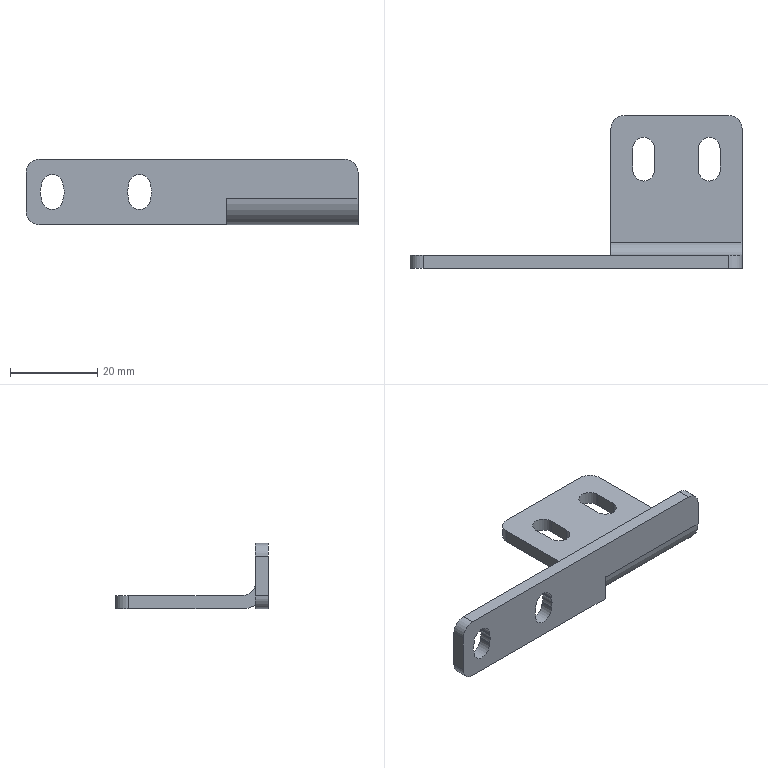Part | NX | features solid 2 | 1 solid | 47 faces | box 76 x 35 x 15 mm | volume 5615 mm3 | plane 24 | cylinder 23 | commonest cylinder face diameters 5 x10 5.5 x6 6 x6 12 x1
STEP:
#1=CARTESIAN_POINT('',(-275.5,-1540.5,1312.));
#2=VERTEX_POINT('',#1);
#3=CARTESIAN_POINT('',(-275.5,-1537.5,1312.));
#4=VERTEX_POINT('',#3);
#5=CARTESIAN_POINT('',(-275.5,-1537.5,1312.));
#6=DIRECTION('',(0.,1.,0.));
#7=VECTOR('',#6,1000.);
#8=LINE('',#5,#7);
#9=EDGE_CURVE('',#2,#4,#8,.T.);
#10=ORIENTED_EDGE('',*,*,#9,.T.);
#11=CARTESIAN_POINT('',(-275.5,-1537.5,1311.646));
#12=VERTEX_POINT('',#11);
#13=CARTESIAN_POINT('',(-275.5,-1537.5,1303.));
#14=DIRECTION('',(0.,0.,1.));
#15=VECTOR('',#14,1000.);
#16=LINE('',#13,#15);
#17=EDGE_CURVE('',#12,#4,#16,.T.);
#18=ORIENTED_EDGE('',*,*,#17,.F.);
#19=CARTESIAN_POINT('',(-275.5,-1540.5,1311.646));
#20=VERTEX_POINT('',#19);
#21=CARTESIAN_POINT('',(-275.5,-1537.5,1311.646));
#22=DIRECTION('',(0.,1.,0.));
#23=VECTOR('',#22,1000.);
#24=LINE('',#21,#23);
#25=EDGE_CURVE('',#20,#12,#24,.T.);
#26=ORIENTED_EDGE('',*,*,#25,.F.);
#27=CARTESIAN_POINT('',(-275.5,-1540.5,1303.));
#28=DIRECTION('',(0.,0.,1.));
#29=VECTOR('',#28,1000.);
#30=LINE('',#27,#29);
#31=EDGE_CURVE('',#20,#2,#30,.T.);
#32=ORIENTED_EDGE('',*,*,#31,.T.);
#33=EDGE_LOOP('',(#10,#18,#26,#32));
#34=FACE_BOUND('',#33,.T.);
#35=CARTESIAN_POINT('',(-275.5,-1537.5,1303.));
#36=DIRECTION('',(1.,0.,0.));
#37=DIRECTION('',(0.,0.,-1.));
#38=AXIS2_PLACEMENT_3D('',#35,#36,#37);
#39=PLANE('',#38);
#40=ADVANCED_FACE('',(#34),#39,.F.);
#41=CARTESIAN_POINT('',(-280.5,-1540.5,1312.));
#42=VERTEX_POINT('',#41);
#43=CARTESIAN_POINT('',(-280.5,-1537.5,1312.));
#44=VERTEX_POINT('',#43);
#45=CARTESIAN_POINT('',(-280.5,-1537.5,1312.));
#46=DIRECTION('',(0.,1.,0.));
#47=VECTOR('',#46,1000.);
#48=LINE('',#45,#47);
#49=EDGE_CURVE('',#42,#44,#48,.T.);
#50=ORIENTED_EDGE('',*,*,#49,.T.);
#51=CARTESIAN_POINT('',(-278.,-1537.5,1312.));
#52=DIRECTION('',(0.,-1.,0.));
#53=DIRECTION('',(-1.,0.,0.));
#54=AXIS2_PLACEMENT_3D('',#51,#52,#53);
#55=CIRCLE('',#54,2.5);
#56=EDGE_CURVE('',#4,#44,#55,.T.);
#57=ORIENTED_EDGE('',*,*,#56,.F.);
#58=ORIENTED_EDGE('',*,*,#9,.F.);
#59=CARTESIAN_POINT('',(-278.,-1540.5,1312.));
#60=DIRECTION('',(0.,-1.,0.));
#61=DIRECTION('',(-1.,0.,0.));
#62=AXIS2_PLACEMENT_3D('',#59,#60,#61);
#63=CIRCLE('',#62,2.5);
#64=EDGE_CURVE('',#2,#42,#63,.T.);
#65=ORIENTED_EDGE('',*,*,#64,.T.);
#66=EDGE_LOOP('',(#50,#57,#58,#65));
#67=FACE_BOUND('',#66,.T.);
#68=CARTESIAN_POINT('',(-278.,-1537.5,1312.));
#69=DIRECTION('',(0.,-1.,0.));
#70=DIRECTION('',(-1.,0.,0.));
#71=AXIS2_PLACEMENT_3D('',#68,#69,#70);
#72=CYLINDRICAL_SURFACE('',#71,2.5);
#73=ADVANCED_FACE('',(#67),#72,.F.);
#74=CARTESIAN_POINT('',(-280.5,-1540.5,1311.646));
#75=VERTEX_POINT('',#74);
#76=CARTESIAN_POINT('',(-280.5,-1537.5,1311.646));
#77=VERTEX_POINT('',#76);
#78=CARTESIAN_POINT('',(-280.5,-1537.5,1311.646));
#79=DIRECTION('',(0.,1.,0.));
#80=VECTOR('',#79,1000.);
#81=LINE('',#78,#80);
#82=EDGE_CURVE('',#75,#77,#81,.T.);
#83=ORIENTED_EDGE('',*,*,#82,.T.);
#84=CARTESIAN_POINT('',(-280.5,-1537.5,1303.));
#85=DIRECTION('',(0.,0.,-1.));
#86=VECTOR('',#85,1000.);
#87=LINE('',#84,#86);
#88=EDGE_CURVE('',#44,#77,#87,.T.);
#89=ORIENTED_EDGE('',*,*,#88,.F.);
#90=ORIENTED_EDGE('',*,*,#49,.F.);
#91=CARTESIAN_POINT('',(-280.5,-1540.5,1303.));
#92=DIRECTION('',(0.,0.,-1.));
#93=VECTOR('',#92,1000.);
#94=LINE('',#91,#93);
#95=EDGE_CURVE('',#42,#75,#94,.T.);
#96=ORIENTED_EDGE('',*,*,#95,.T.);
#97=EDGE_LOOP('',(#83,#89,#90,#96));
#98=FACE_BOUND('',#97,.T.);
#99=CARTESIAN_POINT('',(-280.5,-1537.5,1303.));
#100=DIRECTION('',(-1.,0.,0.));
#101=DIRECTION('',(0.,1.,0.));
#102=AXIS2_PLACEMENT_3D('',#99,#100,#101);
#103=PLANE('',#102);
#104=ADVANCED_FACE('',(#98),#103,.F.);
#105=CARTESIAN_POINT('',(-280.5,-1540.5,1309.));
#106=VERTEX_POINT('',#105);
#107=CARTESIAN_POINT('',(-275.5,-1540.5,1309.));
#108=VERTEX_POINT('',#107);
#109=CARTESIAN_POINT('',(-278.,-1540.5,1309.));
#110=DIRECTION('',(0.,-1.,0.));
#111=DIRECTION('',(-1.,0.,0.));
#112=AXIS2_PLACEMENT_3D('',#109,#110,#111);
#113=CIRCLE('',#112,2.5);
#114=EDGE_CURVE('',#106,#108,#113,.T.);
#115=ORIENTED_EDGE('',*,*,#114,.T.);
#116=CARTESIAN_POINT('',(-275.5,-1537.5,1309.));
#117=VERTEX_POINT('',#116);
#118=CARTESIAN_POINT('',(-275.5,-1537.5,1309.));
#119=DIRECTION('',(0.,1.,0.));
#120=VECTOR('',#119,1000.);
#121=LINE('',#118,#120);
#122=EDGE_CURVE('',#108,#117,#121,.T.);
#123=ORIENTED_EDGE('',*,*,#122,.T.);
#124=CARTESIAN_POINT('',(-280.5,-1537.5,1309.));
#125=VERTEX_POINT('',#124);
#126=CARTESIAN_POINT('',(-278.,-1537.5,1309.));
#127=DIRECTION('',(0.,-1.,0.));
#128=DIRECTION('',(-1.,0.,0.));
#129=AXIS2_PLACEMENT_3D('',#126,#127,#128);
#130=CIRCLE('',#129,2.5);
#131=EDGE_CURVE('',#125,#117,#130,.T.);
#132=ORIENTED_EDGE('',*,*,#131,.F.);
#133=CARTESIAN_POINT('',(-280.5,-1537.5,1309.));
#134=DIRECTION('',(0.,1.,0.));
#135=VECTOR('',#134,1000.);
#136=LINE('',#133,#135);
#137=EDGE_CURVE('',#106,#125,#136,.T.);
#138=ORIENTED_EDGE('',*,*,#137,.F.);
#139=EDGE_LOOP('',(#115,#123,#132,#138));
#140=FACE_BOUND('',#139,.T.);
#141=CARTESIAN_POINT('',(-278.,-1537.5,1309.));
#142=DIRECTION('',(0.,-1.,0.));
#143=DIRECTION('',(-1.,0.,0.));
#144=AXIS2_PLACEMENT_3D('',#141,#142,#143);
#145=CYLINDRICAL_SURFACE('',#144,2.5);
#146=ADVANCED_FACE('',(#140),#145,.F.);
#147=CARTESIAN_POINT('',(-275.5,-1540.5,1309.354));
#148=VERTEX_POINT('',#147);
#149=CARTESIAN_POINT('',(-275.5,-1537.5,1309.354));
#150=VERTEX_POINT('',#149);
#151=CARTESIAN_POINT('',(-275.5,-1537.5,1309.354));
#152=DIRECTION('',(0.,1.,0.));
#153=VECTOR('',#152,1000.);
#154=LINE('',#151,#153);
#155=EDGE_CURVE('',#148,#150,#154,.T.);
#156=ORIENTED_EDGE('',*,*,#155,.T.);
#157=CARTESIAN_POINT('',(-275.5,-1537.5,1303.));
#158=DIRECTION('',(0.,0.,1.));
#159=VECTOR('',#158,1000.);
#160=LINE('',#157,#159);
#161=EDGE_CURVE('',#117,#150,#160,.T.);
#162=ORIENTED_EDGE('',*,*,#161,.F.);
#163=ORIENTED_EDGE('',*,*,#122,.F.);
#164=CARTESIAN_POINT('',(-275.5,-1540.5,1303.));
#165=DIRECTION('',(0.,0.,1.));
#166=VECTOR('',#165,1000.);
#167=LINE('',#164,#166);
#168=EDGE_CURVE('',#108,#148,#167,.T.);
#169=ORIENTED_EDGE('',*,*,#168,.T.);
#170=EDGE_LOOP('',(#156,#162,#163,#169));
#171=FACE_BOUND('',#170,.T.);
#172=CARTESIAN_POINT('',(-275.5,-1537.5,1303.));
#173=DIRECTION('',(1.,0.,0.));
#174=DIRECTION('',(0.,0.,-1.));
#175=AXIS2_PLACEMENT_3D('',#172,#173,#174);
#176=PLANE('',#175);
#177=ADVANCED_FACE('',(#171),#176,.F.);
#178=ORIENTED_EDGE('',*,*,#137,.T.);
#179=CARTESIAN_POINT('',(-280.5,-1537.5,1309.354));
#180=VERTEX_POINT('',#179);
#181=CARTESIAN_POINT('',(-280.5,-1537.5,1303.));
#182=DIRECTION('',(0.,0.,-1.));
#183=VECTOR('',#182,1000.);
#184=LINE('',#181,#183);
#185=EDGE_CURVE('',#180,#125,#184,.T.);
#186=ORIENTED_EDGE('',*,*,#185,.F.);
#187=CARTESIAN_POINT('',(-280.5,-1540.5,1309.354));
#188=VERTEX_POINT('',#187);
#189=CARTESIAN_POINT('',(-280.5,-1537.5,1309.354));
#190=DIRECTION('',(0.,1.,0.));
#191=VECTOR('',#190,1000.);
#192=LINE('',#189,#191);
#193=EDGE_CURVE('',#188,#180,#192,.T.);
#194=ORIENTED_EDGE('',*,*,#193,.F.);
#195=CARTESIAN_POINT('',(-280.5,-1540.5,1303.));
#196=DIRECTION('',(0.,0.,-1.));
#197=VECTOR('',#196,1000.);
#198=LINE('',#195,#197);
#199=EDGE_CURVE('',#188,#106,#198,.T.);
#200=ORIENTED_EDGE('',*,*,#199,.T.);
#201=EDGE_LOOP('',(#178,#186,#194,#200));
#202=FACE_BOUND('',#201,.T.);
#203=CARTESIAN_POINT('',(-280.5,-1537.5,1303.));
#204=DIRECTION('',(-1.,0.,0.));
#205=DIRECTION('',(0.,1.,0.));
#206=AXIS2_PLACEMENT_3D('',#203,#204,#205);
#207=PLANE('',#206);
#208=ADVANCED_FACE('',(#202),#207,.F.);
#209=CARTESIAN_POINT('',(-295.5,-1540.5,1312.));
#210=VERTEX_POINT('',#209);
#211=CARTESIAN_POINT('',(-295.5,-1537.5,1312.));
#212=VERTEX_POINT('',#211);
#213=CARTESIAN_POINT('',(-295.5,-1537.5,1312.));
#214=DIRECTION('',(0.,1.,0.));
#215=VECTOR('',#214,1000.);
#216=LINE('',#213,#215);
#217=EDGE_CURVE('',#210,#212,#216,.T.);
#218=ORIENTED_EDGE('',*,*,#217,.T.);
#219=CARTESIAN_POINT('',(-295.5,-1537.5,1311.646));
#220=VERTEX_POINT('',#219);
#221=CARTESIAN_POINT('',(-295.5,-1537.5,1303.));
#222=DIRECTION('',(0.,0.,1.));
#223=VECTOR('',#222,1000.);
#224=LINE('',#221,#223);
#225=EDGE_CURVE('',#220,#212,#224,.T.);
#226=ORIENTED_EDGE('',*,*,#225,.F.);
#227=CARTESIAN_POINT('',(-295.5,-1540.5,1311.646));
#228=VERTEX_POINT('',#227);
#229=CARTESIAN_POINT('',(-295.5,-1537.5,1311.646));
#230=DIRECTION('',(0.,1.,0.));
#231=VECTOR('',#230,1000.);
#232=LINE('',#229,#231);
#233=EDGE_CURVE('',#228,#220,#232,.T.);
#234=ORIENTED_EDGE('',*,*,#233,.F.);
#235=CARTESIAN_POINT('',(-295.5,-1540.5,1303.));
#236=DIRECTION('',(0.,0.,1.));
#237=VECTOR('',#236,1000.);
#238=LINE('',#235,#237);
#239=EDGE_CURVE('',#228,#210,#238,.T.);
#240=ORIENTED_EDGE('',*,*,#239,.T.);
#241=EDGE_LOOP('',(#218,#226,#234,#240));
#242=FACE_BOUND('',#241,.T.);
#243=CARTESIAN_POINT('',(-295.5,-1537.5,1303.));
#244=DIRECTION('',(1.,0.,0.));
#245=DIRECTION('',(0.,0.,-1.));
#246=AXIS2_PLACEMENT_3D('',#243,#244,#245);
#247=PLANE('',#246);
#248=ADVANCED_FACE('',(#242),#247,.F.);
#249=CARTESIAN_POINT('',(-300.5,-1540.5,1312.));
#250=VERTEX_POINT('',#249);
#251=CARTESIAN_POINT('',(-300.5,-1537.5,1312.));
#252=VERTEX_POINT('',#251);
#253=CARTESIAN_POINT('',(-300.5,-1537.5,1312.));
#254=DIRECTION('',(0.,1.,0.));
#255=VECTOR('',#254,1000.);
#256=LINE('',#253,#255);
#257=EDGE_CURVE('',#250,#252,#256,.T.);
#258=ORIENTED_EDGE('',*,*,#257,.T.);
#259=CARTESIAN_POINT('',(-298.,-1537.5,1312.));
#260=DIRECTION('',(0.,-1.,0.));
#261=DIRECTION('',(-1.,0.,0.));
#262=AXIS2_PLACEMENT_3D('',#259,#260,#261);
#263=CIRCLE('',#262,2.5);
#264=EDGE_CURVE('',#212,#252,#263,.T.);
#265=ORIENTED_EDGE('',*,*,#264,.F.);
#266=ORIENTED_EDGE('',*,*,#217,.F.);
#267=CARTESIAN_POINT('',(-298.,-1540.5,1312.));
#268=DIRECTION('',(0.,-1.,0.));
#269=DIRECTION('',(-1.,0.,0.));
#270=AXIS2_PLACEMENT_3D('',#267,#268,#269);
#271=CIRCLE('',#270,2.5);
#272=EDGE_CURVE('',#210,#250,#271,.T.);
#273=ORIENTED_EDGE('',*,*,#272,.T.);
#274=EDGE_LOOP('',(#258,#265,#266,#273));
#275=FACE_BOUND('',#274,.T.);
#276=CARTESIAN_POINT('',(-298.,-1537.5,1312.));
#277=DIRECTION('',(0.,-1.,0.));
#278=DIRECTION('',(-1.,0.,0.));
#279=AXIS2_PLACEMENT_3D('',#276,#277,#278);
#280=CYLINDRICAL_SURFACE('',#279,2.5);
#281=ADVANCED_FACE('',(#275),#280,.F.);
#282=CARTESIAN_POINT('',(-300.5,-1540.5,1311.646));
#283=VERTEX_POINT('',#282);
#284=CARTESIAN_POINT('',(-300.5,-1537.5,1311.646));
#285=VERTEX_POINT('',#284);
#286=CARTESIAN_POINT('',(-300.5,-1537.5,1311.646));
#287=DIRECTION('',(0.,1.,0.));
#288=VECTOR('',#287,1000.);
#289=LINE('',#286,#288);
#290=EDGE_CURVE('',#283,#285,#289,.T.);
#291=ORIENTED_EDGE('',*,*,#290,.T.);
#292=CARTESIAN_POINT('',(-300.5,-1537.5,1303.));
#293=DIRECTION('',(0.,0.,-1.));
#294=VECTOR('',#293,1000.);
#295=LINE('',#292,#294);
#296=EDGE_CURVE('',#252,#285,#295,.T.);
#297=ORIENTED_EDGE('',*,*,#296,.F.);
#298=ORIENTED_EDGE('',*,*,#257,.F.);
#299=CARTESIAN_POINT('',(-300.5,-1540.5,1303.));
#300=DIRECTION('',(0.,0.,-1.));
#301=VECTOR('',#300,1000.);
#302=LINE('',#299,#301);
#303=EDGE_CURVE('',#250,#283,#302,.T.);
#304=ORIENTED_EDGE('',*,*,#303,.T.);
#305=EDGE_LOOP('',(#291,#297,#298,#304));
#306=FACE_BOUND('',#305,.T.);
#307=CARTESIAN_POINT('',(-300.5,-1537.5,1303.));
#308=DIRECTION('',(-1.,0.,0.));
#309=DIRECTION('',(0.,1.,0.));
#310=AXIS2_PLACEMENT_3D('',#307,#308,#309);
#311=PLANE('',#310);
#312=ADVANCED_FACE('',(#306),#311,.F.);
#313=CARTESIAN_POINT('',(-300.5,-1540.5,1309.));
#314=VERTEX_POINT('',#313);
#315=CARTESIAN_POINT('',(-295.5,-1540.5,1309.));
#316=VERTEX_POINT('',#315);
#317=CARTESIAN_POINT('',(-298.,-1540.5,1309.));
#318=DIRECTION('',(0.,-1.,0.));
#319=DIRECTION('',(-1.,0.,0.));
#320=AXIS2_PLACEMENT_3D('',#317,#318,#319);
#321=CIRCLE('',#320,2.5);
#322=EDGE_CURVE('',#314,#316,#321,.T.);
#323=ORIENTED_EDGE('',*,*,#322,.T.);
#324=CARTESIAN_POINT('',(-295.5,-1537.5,1309.));
#325=VERTEX_POINT('',#324);
#326=CARTESIAN_POINT('',(-295.5,-1537.5,1309.));
#327=DIRECTION('',(0.,1.,0.));
#328=VECTOR('',#327,1000.);
#329=LINE('',#326,#328);
#330=EDGE_CURVE('',#316,#325,#329,.T.);
#331=ORIENTED_EDGE('',*,*,#330,.T.);
#332=CARTESIAN_POINT('',(-300.5,-1537.5,1309.));
#333=VERTEX_POINT('',#332);
#334=CARTESIAN_POINT('',(-298.,-1537.5,1309.));
#335=DIRECTION('',(0.,-1.,0.));
#336=DIRECTION('',(-1.,0.,0.));
#337=AXIS2_PLACEMENT_3D('',#334,#335,#336);
#338=CIRCLE('',#337,2.5);
#339=EDGE_CURVE('',#333,#325,#338,.T.);
#340=ORIENTED_EDGE('',*,*,#339,.F.);
#341=CARTESIAN_POINT('',(-300.5,-1537.5,1309.));
#342=DIRECTION('',(0.,1.,0.));
#343=VECTOR('',#342,1000.);
#344=LINE('',#341,#343);
#345=EDGE_CURVE('',#314,#333,#344,.T.);
#346=ORIENTED_EDGE('',*,*,#345,.F.);
#347=EDGE_LOOP('',(#323,#331,#340,#346));
#348=FACE_BOUND('',#347,.T.);
#349=CARTESIAN_POINT('',(-298.,-1537.5,1309.));
#350=DIRECTION('',(0.,-1.,0.));
#351=DIRECTION('',(-1.,0.,0.));
#352=AXIS2_PLACEMENT_3D('',#349,#350,#351);
#353=CYLINDRICAL_SURFACE('',#352,2.5);
#354=ADVANCED_FACE('',(#348),#353,.F.);
#355=CARTESIAN_POINT('',(-295.5,-1540.5,1309.354));
#356=VERTEX_POINT('',#355);
#357=CARTESIAN_POINT('',(-295.5,-1537.5,1309.354));
#358=VERTEX_POINT('',#357);
#359=CARTESIAN_POINT('',(-295.5,-1537.5,1309.354));
#360=DIRECTION('',(0.,1.,0.));
#361=VECTOR('',#360,1000.);
#362=LINE('',#359,#361);
#363=EDGE_CURVE('',#356,#358,#362,.T.);
#364=ORIENTED_EDGE('',*,*,#363,.T.);
#365=CARTESIAN_POINT('',(-295.5,-1537.5,1303.));
#366=DIRECTION('',(0.,0.,1.));
#367=VECTOR('',#366,1000.);
#368=LINE('',#365,#367);
#369=EDGE_CURVE('',#325,#358,#368,.T.);
#370=ORIENTED_EDGE('',*,*,#369,.F.);
#371=ORIENTED_EDGE('',*,*,#330,.F.);
#372=CARTESIAN_POINT('',(-295.5,-1540.5,1303.));
#373=DIRECTION('',(0.,0.,1.));
#374=VECTOR('',#373,1000.);
#375=LINE('',#372,#374);
#376=EDGE_CURVE('',#316,#356,#375,.T.);
#377=ORIENTED_EDGE('',*,*,#376,.T.);
#378=EDGE_LOOP('',(#364,#370,#371,#377));
#379=FACE_BOUND('',#378,.T.);
#380=CARTESIAN_POINT('',(-295.5,-1537.5,1303.));
#381=DIRECTION('',(1.,0.,0.));
#382=DIRECTION('',(0.,0.,-1.));
#383=AXIS2_PLACEMENT_3D('',#380,#381,#382);
#384=PLANE('',#383);
#385=ADVANCED_FACE('',(#379),#384,.F.);
#386=ORIENTED_EDGE('',*,*,#345,.T.);
#387=CARTESIAN_POINT('',(-300.5,-1537.5,1309.354));
#388=VERTEX_POINT('',#387);
#389=CARTESIAN_POINT('',(-300.5,-1537.5,1303.));
#390=DIRECTION('',(0.,0.,-1.));
#391=VECTOR('',#390,1000.);
#392=LINE('',#389,#391);
#393=EDGE_CURVE('',#388,#333,#392,.T.);
#394=ORIENTED_EDGE('',*,*,#393,.F.);
#395=CARTESIAN_POINT('',(-300.5,-1540.5,1309.354));
#396=VERTEX_POINT('',#395);
#397=CARTESIAN_POINT('',(-300.5,-1537.5,1309.354));
#398=DIRECTION('',(0.,1.,0.));
#399=VECTOR('',#398,1000.);
#400=LINE('',#397,#399);
#401=EDGE_CURVE('',#396,#388,#400,.T.);
#402=ORIENTED_EDGE('',*,*,#401,.F.);
#403=CARTESIAN_POINT('',(-300.5,-1540.5,1303.));
#404=DIRECTION('',(0.,0.,-1.));
#405=VECTOR('',#404,1000.);
#406=LINE('',#403,#405);
#407=EDGE_CURVE('',#396,#314,#406,.T.);
#408=ORIENTED_EDGE('',*,*,#407,.T.);
#409=EDGE_LOOP('',(#386,#394,#402,#408));
#410=FACE_BOUND('',#409,.T.);
#411=CARTESIAN_POINT('',(-300.5,-1537.5,1303.));
#412=DIRECTION('',(-1.,0.,0.));
#413=DIRECTION('',(0.,1.,0.));
#414=AXIS2_PLACEMENT_3D('',#411,#412,#413);
#415=PLANE('',#414);
#416=ADVANCED_FACE('',(#410),#415,.F.);
#417=CARTESIAN_POINT('',(-253.,-1518.,1306.));
#418=VERTEX_POINT('',#417);
#419=CARTESIAN_POINT('',(-253.,-1518.,1303.));
#420=VERTEX_POINT('',#419);
#421=CARTESIAN_POINT('',(-253.,-1518.,1388.006));
#422=DIRECTION('',(0.,0.,-1.));
#423=VECTOR('',#422,1000.);
#424=LINE('',#421,#423);
#425=EDGE_CURVE('',#418,#420,#424,.T.);
#426=ORIENTED_EDGE('',*,*,#425,.T.);
#427=CARTESIAN_POINT('',(-253.,-1513.,1303.));
#428=VERTEX_POINT('',#427);
#429=CARTESIAN_POINT('',(-253.,-1518.,1303.));
#430=DIRECTION('',(0.,1.,0.));
#431=VECTOR('',#430,1000.);
#432=LINE('',#429,#431);
#433=EDGE_CURVE('',#420,#428,#432,.T.);
#434=ORIENTED_EDGE('',*,*,#433,.T.);
#435=CARTESIAN_POINT('',(-253.,-1513.,1306.));
#436=VERTEX_POINT('',#435);
#437=CARTESIAN_POINT('',(-253.,-1513.,1388.006));
#438=DIRECTION('',(0.,0.,-1.));
#439=VECTOR('',#438,1000.);
#440=LINE('',#437,#439);
#441=EDGE_CURVE('',#436,#428,#440,.T.);
#442=ORIENTED_EDGE('',*,*,#441,.F.);
#443=CARTESIAN_POINT('',(-253.,-1540.5,1306.));
#444=DIRECTION('',(0.,1.,0.));
#445=VECTOR('',#444,1000.);
#446=LINE('',#443,#445);
#447=EDGE_CURVE('',#418,#436,#446,.T.);
#448=ORIENTED_EDGE('',*,*,#447,.F.);
#449=EDGE_LOOP('',(#426,#434,#442,#448));
#450=FACE_BOUND('',#449,.T.);
#451=CARTESIAN_POINT('',(-253.,-1518.,1388.006));
#452=DIRECTION('',(-1.,0.,0.));
#453=DIRECTION('',(0.,1.,0.));
#454=AXIS2_PLACEMENT_3D('',#451,#452,#453);
#455=PLANE('',#454);
#456=ADVANCED_FACE('',(#450),#455,.F.);
#457=CARTESIAN_POINT('',(-250.5,-1520.5,1306.));
#458=VERTEX_POINT('',#457);
#459=CARTESIAN_POINT('',(-250.5,-1520.5,1303.));
#460=VERTEX_POINT('',#459);
#461=CARTESIAN_POINT('',(-250.5,-1520.5,1388.006));
#462=DIRECTION('',(0.,0.,-1.));
#463=VECTOR('',#462,1000.);
#464=LINE('',#461,#463);
#465=EDGE_CURVE('',#458,#460,#464,.T.);
#466=ORIENTED_EDGE('',*,*,#465,.F.);
#467=CARTESIAN_POINT('',(-248.,-1518.,1306.));
#468=VERTEX_POINT('',#467);
#469=CARTESIAN_POINT('',(-250.5,-1518.,1306.));
#470=DIRECTION('',(0.,0.,-1.));
#471=DIRECTION('',(0.,-1.,0.));
#472=AXIS2_PLACEMENT_3D('',#469,#470,#471);
#473=CIRCLE('',#472,2.5);
#474=EDGE_CURVE('',#468,#458,#473,.T.);
#475=ORIENTED_EDGE('',*,*,#474,.F.);
#476=CARTESIAN_POINT('',(-248.,-1518.,1303.));
#477=VERTEX_POINT('',#476);
#478=CARTESIAN_POINT('',(-248.,-1518.,1388.006));
#479=DIRECTION('',(0.,0.,-1.));
#480=VECTOR('',#479,1000.);
#481=LINE('',#478,#480);
#482=EDGE_CURVE('',#468,#477,#481,.T.);
#483=ORIENTED_EDGE('',*,*,#482,.T.);
#484=CARTESIAN_POINT('',(-250.5,-1518.,1303.));
#485=DIRECTION('',(0.,0.,-1.));
#486=DIRECTION('',(1.,0.,0.));
#487=AXIS2_PLACEMENT_3D('',#484,#485,#486);
#488=CIRCLE('',#487,2.5);
#489=EDGE_CURVE('',#477,#460,#488,.T.);
#490=ORIENTED_EDGE('',*,*,#489,.T.);
#491=EDGE_LOOP('',(#466,#475,#483,#490));
#492=FACE_BOUND('',#491,.T.);
#493=CARTESIAN_POINT('',(-250.5,-1518.,1388.006));
#494=DIRECTION('',(0.,0.,-1.));
#495=DIRECTION('',(0.,-1.,0.));
#496=AXIS2_PLACEMENT_3D('',#493,#494,#495);
#497=CYLINDRICAL_SURFACE('',#496,2.5);
#498=ADVANCED_FACE('',(#492),#497,.F.);
#499=CARTESIAN_POINT('',(-248.,-1513.,1306.));
#500=VERTEX_POINT('',#499);
#501=CARTESIAN_POINT('',(-248.,-1513.,1303.));
#502=VERTEX_POINT('',#501);
#503=CARTESIAN_POINT('',(-248.,-1513.,1388.006));
#504=DIRECTION('',(0.,0.,-1.));
#505=VECTOR('',#504,1000.);
#506=LINE('',#503,#505);
#507=EDGE_CURVE('',#500,#502,#506,.T.);
#508=ORIENTED_EDGE('',*,*,#507,.T.);
#509=CARTESIAN_POINT('',(-248.,-1518.,1303.));
#510=DIRECTION('',(0.,-1.,0.));
#511=VECTOR('',#510,1000.);
#512=LINE('',#509,#511);
#513=EDGE_CURVE('',#502,#477,#512,.T.);
#514=ORIENTED_EDGE('',*,*,#513,.T.);
#515=ORIENTED_EDGE('',*,*,#482,.F.);
#516=CARTESIAN_POINT('',(-248.,-1540.5,1306.));
#517=DIRECTION('',(0.,-1.,0.));
#518=VECTOR('',#517,1000.);
#519=LINE('',#516,#518);
#520=EDGE_CURVE('',#500,#468,#519,.T.);
#521=ORIENTED_EDGE('',*,*,#520,.F.);
#522=EDGE_LOOP('',(#508,#514,#515,#521));
#523=FACE_BOUND('',#522,.T.);
#524=CARTESIAN_POINT('',(-248.,-1518.,1388.006));
#525=DIRECTION('',(1.,0.,0.));
#526=DIRECTION('',(0.,0.,-1.));
#527=AXIS2_PLACEMENT_3D('',#524,#525,#526);
#528=PLANE('',#527);
#529=ADVANCED_FACE('',(#523),#528,.F.);
#530=ORIENTED_EDGE('',*,*,#441,.T.);
#531=CARTESIAN_POINT('',(-250.5,-1513.,1303.));
#532=DIRECTION('',(0.,0.,-1.));
#533=DIRECTION('',(-1.,0.,0.));
#534=AXIS2_PLACEMENT_3D('',#531,#532,#533);
#535=CIRCLE('',#534,2.5);
#536=EDGE_CURVE('',#428,#502,#535,.T.);
#537=ORIENTED_EDGE('',*,*,#536,.T.);
#538=ORIENTED_EDGE('',*,*,#507,.F.);
#539=CARTESIAN_POINT('',(-250.5,-1513.,1306.));
#540=DIRECTION('',(0.,0.,-1.));
#541=DIRECTION('',(0.,-1.,0.));
#542=AXIS2_PLACEMENT_3D('',#539,#540,#541);
#543=CIRCLE('',#542,2.5);
#544=EDGE_CURVE('',#436,#500,#543,.T.);
#545=ORIENTED_EDGE('',*,*,#544,.F.);
#546=EDGE_LOOP('',(#530,#537,#538,#545));
#547=FACE_BOUND('',#546,.T.);
#548=CARTESIAN_POINT('',(-250.5,-1513.,1388.006));
#549=DIRECTION('',(0.,0.,-1.));
#550=DIRECTION('',(0.,-1.,0.));
#551=AXIS2_PLACEMENT_3D('',#548,#549,#550);
#552=CYLINDRICAL_SURFACE('',#551,2.5);
#553=ADVANCED_FACE('',(#547),#552,.F.);
#554=CARTESIAN_POINT('',(-238.,-1518.,1306.));
#555=VERTEX_POINT('',#554);
#556=CARTESIAN_POINT('',(-238.,-1518.,1303.));
#557=VERTEX_POINT('',#556);
#558=CARTESIAN_POINT('',(-238.,-1518.,1388.006));
#559=DIRECTION('',(0.,0.,-1.));
#560=VECTOR('',#559,1000.);
#561=LINE('',#558,#560);
#562=EDGE_CURVE('',#555,#557,#561,.T.);
#563=ORIENTED_EDGE('',*,*,#562,.T.);
#564=CARTESIAN_POINT('',(-238.,-1513.,1303.));
#565=VERTEX_POINT('',#564);
#566=CARTESIAN_POINT('',(-238.,-1518.,1303.));
#567=DIRECTION('',(0.,1.,0.));
#568=VECTOR('',#567,1000.);
#569=LINE('',#566,#568);
#570=EDGE_CURVE('',#557,#565,#569,.T.);
#571=ORIENTED_EDGE('',*,*,#570,.T.);
#572=CARTESIAN_POINT('',(-238.,-1513.,1306.));
#573=VERTEX_POINT('',#572);
#574=CARTESIAN_POINT('',(-238.,-1513.,1388.006));
#575=DIRECTION('',(0.,0.,-1.));
#576=VECTOR('',#575,1000.);
#577=LINE('',#574,#576);
#578=EDGE_CURVE('',#573,#565,#577,.T.);
#579=ORIENTED_EDGE('',*,*,#578,.F.);
#580=CARTESIAN_POINT('',(-238.,-1540.5,1306.));
#581=DIRECTION('',(0.,1.,0.));
#582=VECTOR('',#581,1000.);
#583=LINE('',#580,#582);
#584=EDGE_CURVE('',#555,#573,#583,.T.);
#585=ORIENTED_EDGE('',*,*,#584,.F.);
#586=EDGE_LOOP('',(#563,#571,#579,#585));
#587=FACE_BOUND('',#586,.T.);
#588=CARTESIAN_POINT('',(-238.,-1518.,1388.006));
#589=DIRECTION('',(-1.,0.,0.));
#590=DIRECTION('',(0.,1.,0.));
#591=AXIS2_PLACEMENT_3D('',#588,#589,#590);
#592=PLANE('',#591);
#593=ADVANCED_FACE('',(#587),#592,.F.);
#594=CARTESIAN_POINT('',(-235.5,-1520.5,1306.));
#595=VERTEX_POINT('',#594);
#596=CARTESIAN_POINT('',(-235.5,-1520.5,1303.));
#597=VERTEX_POINT('',#596);
#598=CARTESIAN_POINT('',(-235.5,-1520.5,1388.006));
#599=DIRECTION('',(0.,0.,-1.));
#600=VECTOR('',#599,1000.);
#601=LINE('',#598,#600);
#602=EDGE_CURVE('',#595,#597,#601,.T.);
#603=ORIENTED_EDGE('',*,*,#602,.F.);
#604=CARTESIAN_POINT('',(-233.,-1518.,1306.));
#605=VERTEX_POINT('',#604);
#606=CARTESIAN_POINT('',(-235.5,-1518.,1306.));
#607=DIRECTION('',(0.,0.,-1.));
#608=DIRECTION('',(0.,-1.,0.));
#609=AXIS2_PLACEMENT_3D('',#606,#607,#608);
#610=CIRCLE('',#609,2.5);
#611=EDGE_CURVE('',#605,#595,#610,.T.);
#612=ORIENTED_EDGE('',*,*,#611,.F.);
#613=CARTESIAN_POINT('',(-233.,-1518.,1303.));
#614=VERTEX_POINT('',#613);
#615=CARTESIAN_POINT('',(-233.,-1518.,1388.006));
#616=DIRECTION('',(0.,0.,-1.));
#617=VECTOR('',#616,1000.);
#618=LINE('',#615,#617);
#619=EDGE_CURVE('',#605,#614,#618,.T.);
#620=ORIENTED_EDGE('',*,*,#619,.T.);
#621=CARTESIAN_POINT('',(-235.5,-1518.,1303.));
#622=DIRECTION('',(0.,0.,-1.));
#623=DIRECTION('',(1.,0.,0.));
#624=AXIS2_PLACEMENT_3D('',#621,#622,#623);
#625=CIRCLE('',#624,2.5);
#626=EDGE_CURVE('',#614,#597,#625,.T.);
#627=ORIENTED_EDGE('',*,*,#626,.T.);
#628=EDGE_LOOP('',(#603,#612,#620,#627));
#629=FACE_BOUND('',#628,.T.);
#630=CARTESIAN_POINT('',(-235.5,-1518.,1388.006));
#631=DIRECTION('',(0.,0.,-1.));
#632=DIRECTION('',(0.,-1.,0.));
#633=AXIS2_PLACEMENT_3D('',#630,#631,#632);
#634=CYLINDRICAL_SURFACE('',#633,2.5);
#635=ADVANCED_FACE('',(#629),#634,.F.);
#636=CARTESIAN_POINT('',(-233.,-1513.,1306.));
#637=VERTEX_POINT('',#636);
#638=CARTESIAN_POINT('',(-233.,-1513.,1303.));
#639=VERTEX_POINT('',#638);
#640=CARTESIAN_POINT('',(-233.,-1513.,1388.006));
#641=DIRECTION('',(0.,0.,-1.));
#642=VECTOR('',#641,1000.);
#643=LINE('',#640,#642);
#644=EDGE_CURVE('',#637,#639,#643,.T.);
#645=ORIENTED_EDGE('',*,*,#644,.T.);
#646=CARTESIAN_POINT('',(-233.,-1518.,1303.));
#647=DIRECTION('',(0.,-1.,0.));
#648=VECTOR('',#647,1000.);
#649=LINE('',#646,#648);
#650=EDGE_CURVE('',#639,#614,#649,.T.);
#651=ORIENTED_EDGE('',*,*,#650,.T.);
#652=ORIENTED_EDGE('',*,*,#619,.F.);
#653=CARTESIAN_POINT('',(-233.,-1540.5,1306.));
#654=DIRECTION('',(0.,-1.,0.));
#655=VECTOR('',#654,1000.);
#656=LINE('',#653,#655);
#657=EDGE_CURVE('',#637,#605,#656,.T.);
#658=ORIENTED_EDGE('',*,*,#657,.F.);
#659=EDGE_LOOP('',(#645,#651,#652,#658));
#660=FACE_BOUND('',#659,.T.);
#661=CARTESIAN_POINT('',(-233.,-1518.,1388.006));
#662=DIRECTION('',(1.,0.,0.));
#663=DIRECTION('',(0.,0.,-1.));
#664=AXIS2_PLACEMENT_3D('',#661,#662,#663);
#665=PLANE('',#664);
#666=ADVANCED_FACE('',(#660),#665,.F.);
#667=ORIENTED_EDGE('',*,*,#578,.T.);
#668=CARTESIAN_POINT('',(-235.5,-1513.,1303.));
#669=DIRECTION('',(0.,0.,-1.));
#670=DIRECTION('',(-1.,0.,0.));
#671=AXIS2_PLACEMENT_3D('',#668,#669,#670);
#672=CIRCLE('',#671,2.5);
#673=EDGE_CURVE('',#565,#639,#672,.T.);
#674=ORIENTED_EDGE('',*,*,#673,.T.);
#675=ORIENTED_EDGE('',*,*,#644,.F.);
#676=CARTESIAN_POINT('',(-235.5,-1513.,1306.));
#677=DIRECTION('',(0.,0.,-1.));
#678=DIRECTION('',(0.,-1.,0.));
#679=AXIS2_PLACEMENT_3D('',#676,#677,#678);
#680=CIRCLE('',#679,2.5);
#681=EDGE_CURVE('',#573,#637,#680,.T.);
#682=ORIENTED_EDGE('',*,*,#681,.F.);
#683=EDGE_LOOP('',(#667,#674,#675,#682));
#684=FACE_BOUND('',#683,.T.);
#685=CARTESIAN_POINT('',(-235.5,-1513.,1388.006));
#686=DIRECTION('',(0.,0.,-1.));
#687=DIRECTION('',(0.,-1.,0.));
#688=AXIS2_PLACEMENT_3D('',#685,#686,#687);
#689=CYLINDRICAL_SURFACE('',#688,2.5);
#690=ADVANCED_FACE('',(#684),#689,.F.);
#691=CARTESIAN_POINT('',(-231.,-1537.5,1318.));
#692=VERTEX_POINT('',#691);
#693=CARTESIAN_POINT('',(-228.,-1537.5,1315.));
#694=VERTEX_POINT('',#693);
#695=CARTESIAN_POINT('',(-231.,-1537.5,1315.));
#696=DIRECTION('',(0.,1.,0.));
#697=DIRECTION('',(-1.,0.,0.));
#698=AXIS2_PLACEMENT_3D('',#695,#696,#697);
#699=CIRCLE('',#698,3.);
#700=EDGE_CURVE('',#692,#694,#699,.T.);
#701=ORIENTED_EDGE('',*,*,#700,.F.);
#702=CARTESIAN_POINT('',(-231.,-1540.5,1318.));
#703=VERTEX_POINT('',#702);
#704=CARTESIAN_POINT('',(-231.,-1537.5,1318.));
#705=DIRECTION('',(0.,1.,0.));
#706=VECTOR('',#705,1000.);
#707=LINE('',#704,#706);
#708=EDGE_CURVE('',#703,#692,#707,.T.);
#709=ORIENTED_EDGE('',*,*,#708,.F.);
#710=CARTESIAN_POINT('',(-228.,-1540.5,1315.));
#711=VERTEX_POINT('',#710);
#712=CARTESIAN_POINT('',(-231.,-1540.5,1315.));
#713=DIRECTION('',(0.,-1.,0.));
#714=DIRECTION('',(-1.,0.,0.));
#715=AXIS2_PLACEMENT_3D('',#712,#713,#714);
#716=CIRCLE('',#715,3.);
#717=EDGE_CURVE('',#711,#703,#716,.T.);
#718=ORIENTED_EDGE('',*,*,#717,.F.);
#719=CARTESIAN_POINT('',(-228.,-1540.5,1315.));
#720=DIRECTION('',(0.,-1.,0.));
#721=VECTOR('',#720,1000.);
#722=LINE('',#719,#721);
#723=EDGE_CURVE('',#694,#711,#722,.T.);
#724=ORIENTED_EDGE('',*,*,#723,.F.);
#725=EDGE_LOOP('',(#701,#709,#718,#724));
#726=FACE_BOUND('',#725,.T.);
#727=CARTESIAN_POINT('',(-231.,-1540.5,1315.));
#728=DIRECTION('',(0.,1.,0.));
#729=DIRECTION('',(1.,0.,0.));
#730=AXIS2_PLACEMENT_3D('',#727,#728,#729);
#731=CYLINDRICAL_SURFACE('',#730,3.);
#732=ADVANCED_FACE('',(#726),#731,.T.);
#733=CARTESIAN_POINT('',(-304.,-1537.5,1315.));
#734=VERTEX_POINT('',#733);
#735=CARTESIAN_POINT('',(-301.,-1537.5,1318.));
#736=VERTEX_POINT('',#735);
#737=CARTESIAN_POINT('',(-301.,-1537.5,1315.));
#738=DIRECTION('',(0.,1.,0.));
#739=DIRECTION('',(-1.,0.,0.));
#740=AXIS2_PLACEMENT_3D('',#737,#738,#739);
#741=CIRCLE('',#740,3.);
#742=EDGE_CURVE('',#734,#736,#741,.T.);
#743=ORIENTED_EDGE('',*,*,#742,.F.);
#744=CARTESIAN_POINT('',(-304.,-1540.5,1315.));
#745=VERTEX_POINT('',#744);
#746=CARTESIAN_POINT('',(-304.,-1540.5,1315.));
#747=DIRECTION('',(0.,1.,0.));
#748=VECTOR('',#747,1000.);
#749=LINE('',#746,#748);
#750=EDGE_CURVE('',#745,#734,#749,.T.);
#751=ORIENTED_EDGE('',*,*,#750,.F.);
#752=CARTESIAN_POINT('',(-301.,-1540.5,1318.));
#753=VERTEX_POINT('',#752);
#754=CARTESIAN_POINT('',(-301.,-1540.5,1315.));
#755=DIRECTION('',(0.,-1.,0.));
#756=DIRECTION('',(-1.,0.,0.));
#757=AXIS2_PLACEMENT_3D('',#754,#755,#756);
#758=CIRCLE('',#757,3.);
#759=EDGE_CURVE('',#753,#745,#758,.T.);
#760=ORIENTED_EDGE('',*,*,#759,.F.);
#761=CARTESIAN_POINT('',(-301.,-1540.5,1318.));
#762=DIRECTION('',(0.,-1.,0.));
#763=VECTOR('',#762,1000.);
#764=LINE('',#761,#763);
#765=EDGE_CURVE('',#736,#753,#764,.T.);
#766=ORIENTED_EDGE('',*,*,#765,.F.);
#767=EDGE_LOOP('',(#743,#751,#760,#766));
#768=FACE_BOUND('',#767,.T.);
#769=CARTESIAN_POINT('',(-301.,-1540.5,1315.));
#770=DIRECTION('',(0.,-1.,0.));
#771=DIRECTION('',(-1.,0.,0.));
#772=AXIS2_PLACEMENT_3D('',#769,#770,#771);
#773=CYLINDRICAL_SURFACE('',#772,3.);
#774=ADVANCED_FACE('',(#768),#773,.T.);
#775=CARTESIAN_POINT('',(-301.,-1537.5,1303.));
#776=VERTEX_POINT('',#775);
#777=CARTESIAN_POINT('',(-304.,-1537.5,1306.));
#778=VERTEX_POINT('',#777);
#779=CARTESIAN_POINT('',(-301.,-1537.5,1306.));
#780=DIRECTION('',(0.,1.,0.));
#781=DIRECTION('',(-1.,0.,0.));
#782=AXIS2_PLACEMENT_3D('',#779,#780,#781);
#783=CIRCLE('',#782,3.);
#784=EDGE_CURVE('',#776,#778,#783,.T.);
#785=ORIENTED_EDGE('',*,*,#784,.F.);
#786=CARTESIAN_POINT('',(-301.,-1540.5,1303.));
#787=VERTEX_POINT('',#786);
#788=CARTESIAN_POINT('',(-301.,-1540.5,1303.));
#789=DIRECTION('',(0.,1.,0.));
#790=VECTOR('',#789,1000.);
#791=LINE('',#788,#790);
#792=EDGE_CURVE('',#787,#776,#791,.T.);
#793=ORIENTED_EDGE('',*,*,#792,.F.);
#794=CARTESIAN_POINT('',(-304.,-1540.5,1306.));
#795=VERTEX_POINT('',#794);
#796=CARTESIAN_POINT('',(-301.,-1540.5,1306.));
#797=DIRECTION('',(0.,-1.,0.));
#798=DIRECTION('',(-1.,0.,0.));
#799=AXIS2_PLACEMENT_3D('',#796,#797,#798);
#800=CIRCLE('',#799,3.);
#801=EDGE_CURVE('',#795,#787,#800,.T.);
#802=ORIENTED_EDGE('',*,*,#801,.F.);
#803=CARTESIAN_POINT('',(-304.,-1540.5,1306.));
#804=DIRECTION('',(0.,-1.,0.));
#805=VECTOR('',#804,1000.);
#806=LINE('',#803,#805);
#807=EDGE_CURVE('',#778,#795,#806,.T.);
#808=ORIENTED_EDGE('',*,*,#807,.F.);
#809=EDGE_LOOP('',(#785,#793,#802,#808));
#810=FACE_BOUND('',#809,.T.);
#811=CARTESIAN_POINT('',(-301.,-1540.5,1306.));
#812=DIRECTION('',(0.,1.,0.));
#813=DIRECTION('',(1.,0.,0.));
#814=AXIS2_PLACEMENT_3D('',#811,#812,#813);
#815=CYLINDRICAL_SURFACE('',#814,3.);
#816=ADVANCED_FACE('',(#810),#815,.T.);
#817=CARTESIAN_POINT('',(-231.,-1505.5,1303.));
#818=VERTEX_POINT('',#817);
#819=CARTESIAN_POINT('',(-228.,-1508.5,1303.));
#820=VERTEX_POINT('',#819);
#821=CARTESIAN_POINT('',(-231.,-1508.5,1303.));
#822=DIRECTION('',(0.,0.,-1.));
#823=DIRECTION('',(0.,-1.,0.));
#824=AXIS2_PLACEMENT_3D('',#821,#822,#823);
#825=CIRCLE('',#824,3.);
#826=EDGE_CURVE('',#818,#820,#825,.T.);
#827=ORIENTED_EDGE('',*,*,#826,.F.);
#828=CARTESIAN_POINT('',(-231.,-1505.5,1306.));
#829=VERTEX_POINT('',#828);
#830=CARTESIAN_POINT('',(-231.,-1505.5,1303.));
#831=DIRECTION('',(0.,0.,-1.));
#832=VECTOR('',#831,1000.);
#833=LINE('',#830,#832);
#834=EDGE_CURVE('',#829,#818,#833,.T.);
#835=ORIENTED_EDGE('',*,*,#834,.F.);
#836=CARTESIAN_POINT('',(-228.,-1508.5,1306.));
#837=VERTEX_POINT('',#836);
#838=CARTESIAN_POINT('',(-231.,-1508.5,1306.));
#839=DIRECTION('',(0.,0.,1.));
#840=DIRECTION('',(0.,-1.,0.));
#841=AXIS2_PLACEMENT_3D('',#838,#839,#840);
#842=CIRCLE('',#841,3.);
#843=EDGE_CURVE('',#837,#829,#842,.T.);
#844=ORIENTED_EDGE('',*,*,#843,.F.);
#845=CARTESIAN_POINT('',(-228.,-1508.5,1303.));
#846=DIRECTION('',(0.,0.,1.));
#847=VECTOR('',#846,1000.);
#848=LINE('',#845,#847);
#849=EDGE_CURVE('',#820,#837,#848,.T.);
#850=ORIENTED_EDGE('',*,*,#849,.F.);
#851=EDGE_LOOP('',(#827,#835,#844,#850));
#852=FACE_BOUND('',#851,.T.);
#853=CARTESIAN_POINT('',(-231.,-1508.5,1303.));
#854=DIRECTION('',(0.,0.,-1.));
#855=DIRECTION('',(-1.,0.,0.));
#856=AXIS2_PLACEMENT_3D('',#853,#854,#855);
#857=CYLINDRICAL_SURFACE('',#856,3.);
#858=ADVANCED_FACE('',(#852),#857,.T.);
#859=CARTESIAN_POINT('',(-258.,-1508.5,1303.));
#860=VERTEX_POINT('',#859);
#861=CARTESIAN_POINT('',(-255.,-1505.5,1303.));
#862=VERTEX_POINT('',#861);
#863=CARTESIAN_POINT('',(-255.,-1508.5,1303.));
#864=DIRECTION('',(0.,0.,-1.));
#865=DIRECTION('',(0.,-1.,0.));
#866=AXIS2_PLACEMENT_3D('',#863,#864,#865);
#867=CIRCLE('',#866,3.);
#868=EDGE_CURVE('',#860,#862,#867,.T.);
#869=ORIENTED_EDGE('',*,*,#868,.F.);
#870=CARTESIAN_POINT('',(-258.,-1508.5,1306.));
#871=VERTEX_POINT('',#870);
#872=CARTESIAN_POINT('',(-258.,-1508.5,1303.));
#873=DIRECTION('',(0.,0.,-1.));
#874=VECTOR('',#873,1000.);
#875=LINE('',#872,#874);
#876=EDGE_CURVE('',#871,#860,#875,.T.);
#877=ORIENTED_EDGE('',*,*,#876,.F.);
#878=CARTESIAN_POINT('',(-255.,-1505.5,1306.));
#879=VERTEX_POINT('',#878);
#880=CARTESIAN_POINT('',(-255.,-1508.5,1306.));
#881=DIRECTION('',(0.,0.,1.));
#882=DIRECTION('',(0.,-1.,0.));
#883=AXIS2_PLACEMENT_3D('',#880,#881,#882);
#884=CIRCLE('',#883,3.);
#885=EDGE_CURVE('',#879,#871,#884,.T.);
#886=ORIENTED_EDGE('',*,*,#885,.F.);
#887=CARTESIAN_POINT('',(-255.,-1505.5,1303.));
#888=DIRECTION('',(0.,0.,1.));
#889=VECTOR('',#888,1000.);
#890=LINE('',#887,#889);
#891=EDGE_CURVE('',#862,#879,#890,.T.);
#892=ORIENTED_EDGE('',*,*,#891,.F.);
#893=EDGE_LOOP('',(#869,#877,#886,#892));
#894=FACE_BOUND('',#893,.T.);
#895=CARTESIAN_POINT('',(-255.,-1508.5,1303.));
#896=DIRECTION('',(0.,0.,1.));
#897=DIRECTION('',(0.,1.,0.));
#898=AXIS2_PLACEMENT_3D('',#895,#896,#897);
#899=CYLINDRICAL_SURFACE('',#898,3.);
#900=ADVANCED_FACE('',(#894),#899,.T.);
#901=CARTESIAN_POINT('',(-258.,-1537.5,1309.));
#902=VERTEX_POINT('',#901);
#903=CARTESIAN_POINT('',(-228.,-1537.5,1309.));
#904=VERTEX_POINT('',#903);
#905=CARTESIAN_POINT('',(-258.,-1537.5,1309.));
#906=DIRECTION('',(1.,0.,0.));
#907=VECTOR('',#906,1000.);
#908=LINE('',#905,#907);
#909=EDGE_CURVE('',#902,#904,#908,.T.);
#910=ORIENTED_EDGE('',*,*,#909,.T.);
#911=CARTESIAN_POINT('',(-228.,-1534.5,1306.));
#912=VERTEX_POINT('',#911);
#913=CARTESIAN_POINT('',(-228.,-1534.5,1309.));
#914=DIRECTION('',(-1.,0.,0.));
#915=DIRECTION('',(0.,0.,-1.));
#916=AXIS2_PLACEMENT_3D('',#913,#914,#915);
#917=CIRCLE('',#916,3.);
#918=EDGE_CURVE('',#912,#904,#917,.T.);
#919=ORIENTED_EDGE('',*,*,#918,.F.);
#920=CARTESIAN_POINT('',(-258.,-1534.5,1306.));
#921=VERTEX_POINT('',#920);
#922=CARTESIAN_POINT('',(-228.,-1534.5,1306.));
#923=DIRECTION('',(-1.,0.,0.));
#924=VECTOR('',#923,1000.);
#925=LINE('',#922,#924);
#926=EDGE_CURVE('',#912,#921,#925,.T.);
#927=ORIENTED_EDGE('',*,*,#926,.T.);
#928=CARTESIAN_POINT('',(-258.,-1534.5,1309.));
#929=DIRECTION('',(-1.,0.,0.));
#930=DIRECTION('',(0.,0.,-1.));
#931=AXIS2_PLACEMENT_3D('',#928,#929,#930);
#932=CIRCLE('',#931,3.);
#933=EDGE_CURVE('',#921,#902,#932,.T.);
#934=ORIENTED_EDGE('',*,*,#933,.T.);
#935=EDGE_LOOP('',(#910,#919,#927,#934));
#936=FACE_BOUND('',#935,.T.);
#937=CARTESIAN_POINT('',(-258.,-1534.5,1309.));
#938=DIRECTION('',(1.,0.,0.));
#939=DIRECTION('',(0.,1.,0.));
#940=AXIS2_PLACEMENT_3D('',#937,#938,#939);
#941=CYLINDRICAL_SURFACE('',#940,3.);
#942=ADVANCED_FACE('',(#936),#941,.F.);
#943=CARTESIAN_POINT('',(-258.,-1540.5,1309.));
#944=VERTEX_POINT('',#943);
#945=CARTESIAN_POINT('',(-228.,-1540.5,1309.));
#946=VERTEX_POINT('',#945);
#947=CARTESIAN_POINT('',(-258.,-1540.5,1309.));
#948=DIRECTION('',(1.,0.,0.));
#949=VECTOR('',#948,1000.);
#950=LINE('',#947,#949);
#951=EDGE_CURVE('',#944,#946,#950,.T.);
#952=ORIENTED_EDGE('',*,*,#951,.F.);
#953=CARTESIAN_POINT('',(-258.,-1534.5,1303.));
#954=VERTEX_POINT('',#953);
#955=CARTESIAN_POINT('',(-258.,-1534.5,1309.));
#956=DIRECTION('',(-1.,0.,0.));
#957=DIRECTION('',(0.,1.,0.));
#958=AXIS2_PLACEMENT_3D('',#955,#956,#957);
#959=CIRCLE('',#958,6.);
#960=EDGE_CURVE('',#954,#944,#959,.T.);
#961=ORIENTED_EDGE('',*,*,#960,.F.);
#962=CARTESIAN_POINT('',(-228.,-1534.5,1303.));
#963=VERTEX_POINT('',#962);
#964=CARTESIAN_POINT('',(-228.,-1534.5,1303.));
#965=DIRECTION('',(-1.,0.,0.));
#966=VECTOR('',#965,1000.);
#967=LINE('',#964,#966);
#968=EDGE_CURVE('',#963,#954,#967,.T.);
#969=ORIENTED_EDGE('',*,*,#968,.F.);
#970=CARTESIAN_POINT('',(-228.,-1534.5,1309.));
#971=DIRECTION('',(-1.,0.,0.));
#972=DIRECTION('',(0.,1.,0.));
#973=AXIS2_PLACEMENT_3D('',#970,#971,#972);
#974=CIRCLE('',#973,6.);
#975=EDGE_CURVE('',#963,#946,#974,.T.);
#976=ORIENTED_EDGE('',*,*,#975,.T.);
#977=EDGE_LOOP('',(#952,#961,#969,#976));
#978=FACE_BOUND('',#977,.T.);
#979=CARTESIAN_POINT('',(-258.,-1534.5,1309.));
#980=DIRECTION('',(1.,0.,0.));
#981=DIRECTION('',(0.,1.,0.));
#982=AXIS2_PLACEMENT_3D('',#979,#980,#981);
#983=CYLINDRICAL_SURFACE('',#982,6.);
#984=ADVANCED_FACE('',(#978),#983,.T.);
#985=CARTESIAN_POINT('',(-258.,-1505.5,1303.));
#986=DIRECTION('',(1.,0.,0.));
#987=VECTOR('',#986,1000.);
#988=LINE('',#985,#987);
#989=EDGE_CURVE('',#862,#818,#988,.T.);
#990=ORIENTED_EDGE('',*,*,#989,.F.);
#991=ORIENTED_EDGE('',*,*,#891,.T.);
#992=CARTESIAN_POINT('',(-258.,-1505.5,1306.));
#993=DIRECTION('',(1.,0.,0.));
#994=VECTOR('',#993,1000.);
#995=LINE('',#992,#994);
#996=EDGE_CURVE('',#879,#829,#995,.T.);
#997=ORIENTED_EDGE('',*,*,#996,.T.);
#998=ORIENTED_EDGE('',*,*,#834,.T.);
#999=EDGE_LOOP('',(#990,#991,#997,#998));
#1000=FACE_BOUND('',#999,.T.);
#1001=CARTESIAN_POINT('',(-258.,-1505.5,1303.));
#1002=DIRECTION('',(0.,-1.,0.));
#1003=DIRECTION('',(-1.,0.,0.));
#1004=AXIS2_PLACEMENT_3D('',#1001,#1002,#1003);
#1005=PLANE('',#1004);
#1006=ADVANCED_FACE('',(#1000),#1005,.F.);
#1007=ORIENTED_EDGE('',*,*,#584,.T.);
#1008=ORIENTED_EDGE('',*,*,#681,.T.);
#1009=ORIENTED_EDGE('',*,*,#657,.T.);
#1010=ORIENTED_EDGE('',*,*,#611,.T.);
#1011=CARTESIAN_POINT('',(-235.5,-1518.,1306.));
#1012=DIRECTION('',(0.,0.,-1.));
#1013=DIRECTION('',(0.,-1.,0.));
#1014=AXIS2_PLACEMENT_3D('',#1011,#1012,#1013);
#1015=CIRCLE('',#1014,2.5);
#1016=EDGE_CURVE('',#595,#555,#1015,.T.);
#1017=ORIENTED_EDGE('',*,*,#1016,.T.);
#1018=EDGE_LOOP('',(#1007,#1008,#1009,#1010,#1017));
#1019=FACE_BOUND('',#1018,.T.);
#1020=ORIENTED_EDGE('',*,*,#447,.T.);
#1021=ORIENTED_EDGE('',*,*,#544,.T.);
#1022=ORIENTED_EDGE('',*,*,#520,.T.);
#1023=ORIENTED_EDGE('',*,*,#474,.T.);
#1024=CARTESIAN_POINT('',(-250.5,-1518.,1306.));
#1025=DIRECTION('',(0.,0.,-1.));
#1026=DIRECTION('',(0.,-1.,0.));
#1027=AXIS2_PLACEMENT_3D('',#1024,#1025,#1026);
#1028=CIRCLE('',#1027,2.5);
#1029=EDGE_CURVE('',#458,#418,#1028,.T.);
#1030=ORIENTED_EDGE('',*,*,#1029,.T.);
#1031=EDGE_LOOP('',(#1020,#1021,#1022,#1023,#1030));
#1032=FACE_BOUND('',#1031,.T.);
#1033=ORIENTED_EDGE('',*,*,#996,.F.);
#1034=ORIENTED_EDGE('',*,*,#885,.T.);
#1035=CARTESIAN_POINT('',(-258.,-1537.987,1306.));
#1036=DIRECTION('',(0.,1.,0.));
#1037=VECTOR('',#1036,1000.);
#1038=LINE('',#1035,#1037);
#1039=EDGE_CURVE('',#921,#871,#1038,.T.);
#1040=ORIENTED_EDGE('',*,*,#1039,.F.);
#1041=ORIENTED_EDGE('',*,*,#926,.F.);
#1042=CARTESIAN_POINT('',(-228.,-1537.987,1306.));
#1043=DIRECTION('',(0.,-1.,0.));
#1044=VECTOR('',#1043,1000.);
#1045=LINE('',#1042,#1044);
#1046=EDGE_CURVE('',#837,#912,#1045,.T.);
#1047=ORIENTED_EDGE('',*,*,#1046,.F.);
#1048=ORIENTED_EDGE('',*,*,#843,.T.);
#1049=EDGE_LOOP('',(#1033,#1034,#1040,#1041,#1047,#1048));
#1050=FACE_BOUND('',#1049,.T.);
#1051=CARTESIAN_POINT('',(-204.,-1540.5,1306.));
#1052=DIRECTION('',(0.,0.,-1.));
#1053=DIRECTION('',(0.,-1.,0.));
#1054=AXIS2_PLACEMENT_3D('',#1051,#1052,#1053);
#1055=PLANE('',#1054);
#1056=ADVANCED_FACE('',(#1019,#1032,#1050),#1055,.F.);
#1057=ORIENTED_EDGE('',*,*,#673,.F.);
#1058=ORIENTED_EDGE('',*,*,#570,.F.);
#1059=CARTESIAN_POINT('',(-235.5,-1518.,1303.));
#1060=DIRECTION('',(0.,0.,-1.));
#1061=DIRECTION('',(1.,0.,0.));
#1062=AXIS2_PLACEMENT_3D('',#1059,#1060,#1061);
#1063=CIRCLE('',#1062,2.5);
#1064=EDGE_CURVE('',#597,#557,#1063,.T.);
#1065=ORIENTED_EDGE('',*,*,#1064,.F.);
#1066=ORIENTED_EDGE('',*,*,#626,.F.);
#1067=ORIENTED_EDGE('',*,*,#650,.F.);
#1068=EDGE_LOOP('',(#1057,#1058,#1065,#1066,#1067));
#1069=FACE_BOUND('',#1068,.T.);
#1070=ORIENTED_EDGE('',*,*,#536,.F.);
#1071=ORIENTED_EDGE('',*,*,#433,.F.);
#1072=CARTESIAN_POINT('',(-250.5,-1518.,1303.));
#1073=DIRECTION('',(0.,0.,-1.));
#1074=DIRECTION('',(1.,0.,0.));
#1075=AXIS2_PLACEMENT_3D('',#1072,#1073,#1074);
#1076=CIRCLE('',#1075,2.5);
#1077=EDGE_CURVE('',#460,#420,#1076,.T.);
#1078=ORIENTED_EDGE('',*,*,#1077,.F.);
#1079=ORIENTED_EDGE('',*,*,#489,.F.);
#1080=ORIENTED_EDGE('',*,*,#513,.F.);
#1081=EDGE_LOOP('',(#1070,#1071,#1078,#1079,#1080));
#1082=FACE_BOUND('',#1081,.T.);
#1083=CARTESIAN_POINT('',(-258.,-1537.987,1303.));
#1084=DIRECTION('',(0.,1.,0.));
#1085=VECTOR('',#1084,1000.);
#1086=LINE('',#1083,#1085);
#1087=EDGE_CURVE('',#954,#860,#1086,.T.);
#1088=ORIENTED_EDGE('',*,*,#1087,.T.);
#1089=ORIENTED_EDGE('',*,*,#868,.T.);
#1090=ORIENTED_EDGE('',*,*,#989,.T.);
#1091=ORIENTED_EDGE('',*,*,#826,.T.);
#1092=CARTESIAN_POINT('',(-228.,-1537.987,1303.));
#1093=DIRECTION('',(0.,-1.,0.));
#1094=VECTOR('',#1093,1000.);
#1095=LINE('',#1092,#1094);
#1096=EDGE_CURVE('',#820,#963,#1095,.T.);
#1097=ORIENTED_EDGE('',*,*,#1096,.T.);
#1098=ORIENTED_EDGE('',*,*,#968,.T.);
#1099=EDGE_LOOP('',(#1088,#1089,#1090,#1091,#1097,#1098));
#1100=FACE_BOUND('',#1099,.T.);
#1101=CARTESIAN_POINT('',(-204.,-1540.5,1303.));
#1102=DIRECTION('',(0.,0.,-1.));
#1103=DIRECTION('',(0.,-1.,0.));
#1104=AXIS2_PLACEMENT_3D('',#1101,#1102,#1103);
#1105=PLANE('',#1104);
#1106=ADVANCED_FACE('',(#1069,#1082,#1100),#1105,.T.);
#1107=CARTESIAN_POINT('',(-258.,-1537.5,1309.1));
#1108=VERTEX_POINT('',#1107);
#1109=CARTESIAN_POINT('',(-258.1,-1537.5,1309.1));
#1110=VERTEX_POINT('',#1109);
#1111=CARTESIAN_POINT('',(-258.,-1537.5,1309.1));
#1112=DIRECTION('',(-1.,0.,0.));
#1113=VECTOR('',#1112,1000.);
#1114=LINE('',#1111,#1113);
#1115=EDGE_CURVE('',#1108,#1110,#1114,.T.);
#1116=ORIENTED_EDGE('',*,*,#1115,.F.);
#1117=CARTESIAN_POINT('',(-258.,-1540.5,1309.1));
#1118=VERTEX_POINT('',#1117);
#1119=CARTESIAN_POINT('',(-258.,-1540.5,1309.1));
#1120=DIRECTION('',(0.,-1.,0.));
#1121=VECTOR('',#1120,1000.);
#1122=LINE('',#1119,#1121);
#1123=EDGE_CURVE('',#1108,#1118,#1122,.T.);
#1124=ORIENTED_EDGE('',*,*,#1123,.T.);
#1125=CARTESIAN_POINT('',(-258.1,-1540.5,1309.1));
#1126=VERTEX_POINT('',#1125);
#1127=CARTESIAN_POINT('',(-258.1,-1540.5,1309.1));
#1128=DIRECTION('',(-1.,0.,0.));
#1129=VECTOR('',#1128,1000.);
#1130=LINE('',#1127,#1129);
#1131=EDGE_CURVE('',#1118,#1126,#1130,.T.);
#1132=ORIENTED_EDGE('',*,*,#1131,.T.);
#1133=CARTESIAN_POINT('',(-258.1,-1540.5,1309.1));
#1134=DIRECTION('',(0.,-1.,0.));
#1135=VECTOR('',#1134,1000.);
#1136=LINE('',#1133,#1135);
#1137=EDGE_CURVE('',#1110,#1126,#1136,.T.);
#1138=ORIENTED_EDGE('',*,*,#1137,.F.);
#1139=EDGE_LOOP('',(#1116,#1124,#1132,#1138));
#1140=FACE_BOUND('',#1139,.T.);
#1141=CARTESIAN_POINT('',(-258.1,-1540.5,1309.1));
#1142=DIRECTION('',(0.,0.,1.));
#1143=DIRECTION('',(0.,-1.,0.));
#1144=AXIS2_PLACEMENT_3D('',#1141,#1142,#1143);
#1145=PLANE('',#1144);
#1146=ADVANCED_FACE('',(#1140),#1145,.F.);
#1147=ORIENTED_EDGE('',*,*,#1137,.T.);
#1148=CARTESIAN_POINT('',(-258.1,-1540.5,1303.));
#1149=VERTEX_POINT('',#1148);
#1150=CARTESIAN_POINT('',(-258.1,-1540.5,1303.));
#1151=DIRECTION('',(0.,0.,-1.));
#1152=VECTOR('',#1151,1000.);
#1153=LINE('',#1150,#1152);
#1154=EDGE_CURVE('',#1126,#1149,#1153,.T.);
#1155=ORIENTED_EDGE('',*,*,#1154,.T.);
#1156=CARTESIAN_POINT('',(-258.1,-1537.5,1303.));
#1157=VERTEX_POINT('',#1156);
#1158=CARTESIAN_POINT('',(-258.1,-1540.5,1303.));
#1159=DIRECTION('',(0.,-1.,0.));
#1160=VECTOR('',#1159,1000.);
#1161=LINE('',#1158,#1160);
#1162=EDGE_CURVE('',#1157,#1149,#1161,.T.);
#1163=ORIENTED_EDGE('',*,*,#1162,.F.);
#1164=CARTESIAN_POINT('',(-258.1,-1537.5,1309.1));
#1165=DIRECTION('',(0.,0.,-1.));
#1166=VECTOR('',#1165,1000.);
#1167=LINE('',#1164,#1166);
#1168=EDGE_CURVE('',#1110,#1157,#1167,.T.);
#1169=ORIENTED_EDGE('',*,*,#1168,.F.);
#1170=EDGE_LOOP('',(#1147,#1155,#1163,#1169));
#1171=FACE_BOUND('',#1170,.T.);
#1172=CARTESIAN_POINT('',(-258.1,-1540.5,1303.));
#1173=DIRECTION('',(-1.,0.,0.));
#1174=DIRECTION('',(0.,1.,0.));
#1175=AXIS2_PLACEMENT_3D('',#1172,#1173,#1174);
#1176=PLANE('',#1175);
#1177=ADVANCED_FACE('',(#1171),#1176,.F.);
#1178=CARTESIAN_POINT('',(-275.25,-1537.5,1310.5));
#1179=VERTEX_POINT('',#1178);
#1180=CARTESIAN_POINT('',(-275.25,-1540.5,1310.5));
#1181=VERTEX_POINT('',#1180);
#1182=CARTESIAN_POINT('',(-275.25,-1537.5,1310.5));
#1183=DIRECTION('',(0.,-1.,0.));
#1184=VECTOR('',#1183,1000.);
#1185=LINE('',#1182,#1184);
#1186=EDGE_CURVE('',#1179,#1181,#1185,.T.);
#1187=ORIENTED_EDGE('',*,*,#1186,.F.);
#1188=CARTESIAN_POINT('',(-278.,-1537.5,1310.5));
#1189=DIRECTION('',(0.,-1.,0.));
#1190=DIRECTION('',(1.,0.,0.));
#1191=AXIS2_PLACEMENT_3D('',#1188,#1189,#1190);
#1192=CIRCLE('',#1191,2.75);
#1193=EDGE_CURVE('',#150,#1179,#1192,.T.);
#1194=ORIENTED_EDGE('',*,*,#1193,.F.);
#1195=ORIENTED_EDGE('',*,*,#155,.F.);
#1196=CARTESIAN_POINT('',(-278.,-1540.5,1310.5));
#1197=DIRECTION('',(0.,-1.,0.));
#1198=DIRECTION('',(-1.,0.,0.));
#1199=AXIS2_PLACEMENT_3D('',#1196,#1197,#1198);
#1200=CIRCLE('',#1199,2.75);
#1201=EDGE_CURVE('',#148,#1181,#1200,.T.);
#1202=ORIENTED_EDGE('',*,*,#1201,.T.);
#1203=EDGE_LOOP('',(#1187,#1194,#1195,#1202));
#1204=FACE_BOUND('',#1203,.T.);
#1205=CARTESIAN_POINT('',(-278.,-1537.5,1310.5));
#1206=DIRECTION('',(0.,-1.,0.));
#1207=DIRECTION('',(1.,0.,0.));
#1208=AXIS2_PLACEMENT_3D('',#1205,#1206,#1207);
#1209=CYLINDRICAL_SURFACE('',#1208,2.75);
#1210=ADVANCED_FACE('',(#1204),#1209,.F.);
#1211=CARTESIAN_POINT('',(-295.25,-1537.5,1310.5));
#1212=VERTEX_POINT('',#1211);
#1213=CARTESIAN_POINT('',(-295.25,-1540.5,1310.5));
#1214=VERTEX_POINT('',#1213);
#1215=CARTESIAN_POINT('',(-295.25,-1537.5,1310.5));
#1216=DIRECTION('',(0.,-1.,0.));
#1217=VECTOR('',#1216,1000.);
#1218=LINE('',#1215,#1217);
#1219=EDGE_CURVE('',#1212,#1214,#1218,.T.);
#1220=ORIENTED_EDGE('',*,*,#1219,.F.);
#1221=CARTESIAN_POINT('',(-298.,-1537.5,1310.5));
#1222=DIRECTION('',(0.,-1.,0.));
#1223=DIRECTION('',(1.,0.,0.));
#1224=AXIS2_PLACEMENT_3D('',#1221,#1222,#1223);
#1225=CIRCLE('',#1224,2.75);
#1226=EDGE_CURVE('',#358,#1212,#1225,.T.);
#1227=ORIENTED_EDGE('',*,*,#1226,.F.);
#1228=ORIENTED_EDGE('',*,*,#363,.F.);
#1229=CARTESIAN_POINT('',(-298.,-1540.5,1310.5));
#1230=DIRECTION('',(0.,-1.,0.));
#1231=DIRECTION('',(-1.,0.,0.));
#1232=AXIS2_PLACEMENT_3D('',#1229,#1230,#1231);
#1233=CIRCLE('',#1232,2.75);
#1234=EDGE_CURVE('',#356,#1214,#1233,.T.);
#1235=ORIENTED_EDGE('',*,*,#1234,.T.);
#1236=EDGE_LOOP('',(#1220,#1227,#1228,#1235));
#1237=FACE_BOUND('',#1236,.T.);
#1238=CARTESIAN_POINT('',(-298.,-1537.5,1310.5));
#1239=DIRECTION('',(0.,-1.,0.));
#1240=DIRECTION('',(1.,0.,0.));
#1241=AXIS2_PLACEMENT_3D('',#1238,#1239,#1240);
#1242=CYLINDRICAL_SURFACE('',#1241,2.75);
#1243=ADVANCED_FACE('',(#1237),#1242,.F.);
#1244=ORIENTED_EDGE('',*,*,#264,.T.);
#1245=ORIENTED_EDGE('',*,*,#296,.T.);
#1246=CARTESIAN_POINT('',(-298.,-1537.5,1310.5));
#1247=DIRECTION('',(0.,-1.,0.));
#1248=DIRECTION('',(1.,0.,0.));
#1249=AXIS2_PLACEMENT_3D('',#1246,#1247,#1248);
#1250=CIRCLE('',#1249,2.75);
#1251=EDGE_CURVE('',#285,#388,#1250,.T.);
#1252=ORIENTED_EDGE('',*,*,#1251,.T.);
#1253=ORIENTED_EDGE('',*,*,#393,.T.);
#1254=ORIENTED_EDGE('',*,*,#339,.T.);
#1255=ORIENTED_EDGE('',*,*,#369,.T.);
#1256=ORIENTED_EDGE('',*,*,#1226,.T.);
#1257=CARTESIAN_POINT('',(-298.,-1537.5,1310.5));
#1258=DIRECTION('',(0.,-1.,0.));
#1259=DIRECTION('',(1.,0.,0.));
#1260=AXIS2_PLACEMENT_3D('',#1257,#1258,#1259);
#1261=CIRCLE('',#1260,2.75);
#1262=EDGE_CURVE('',#1212,#220,#1261,.T.);
#1263=ORIENTED_EDGE('',*,*,#1262,.T.);
#1264=ORIENTED_EDGE('',*,*,#225,.T.);
#1265=EDGE_LOOP('',(#1244,#1245,#1252,#1253,#1254,#1255,#1256,#1263,#1264));
#1266=FACE_BOUND('',#1265,.T.);
#1267=ORIENTED_EDGE('',*,*,#56,.T.);
#1268=ORIENTED_EDGE('',*,*,#88,.T.);
#1269=CARTESIAN_POINT('',(-278.,-1537.5,1310.5));
#1270=DIRECTION('',(0.,-1.,0.));
#1271=DIRECTION('',(1.,0.,0.));
#1272=AXIS2_PLACEMENT_3D('',#1269,#1270,#1271);
#1273=CIRCLE('',#1272,2.75);
#1274=EDGE_CURVE('',#77,#180,#1273,.T.);
#1275=ORIENTED_EDGE('',*,*,#1274,.T.);
#1276=ORIENTED_EDGE('',*,*,#185,.T.);
#1277=ORIENTED_EDGE('',*,*,#131,.T.);
#1278=ORIENTED_EDGE('',*,*,#161,.T.);
#1279=ORIENTED_EDGE('',*,*,#1193,.T.);
#1280=CARTESIAN_POINT('',(-278.,-1537.5,1310.5));
#1281=DIRECTION('',(0.,-1.,0.));
#1282=DIRECTION('',(1.,0.,0.));
#1283=AXIS2_PLACEMENT_3D('',#1280,#1281,#1282);
#1284=CIRCLE('',#1283,2.75);
#1285=EDGE_CURVE('',#1179,#12,#1284,.T.);
#1286=ORIENTED_EDGE('',*,*,#1285,.T.);
#1287=ORIENTED_EDGE('',*,*,#17,.T.);
#1288=EDGE_LOOP('',(#1267,#1268,#1275,#1276,#1277,#1278,#1279,#1286,#1287));
#1289=FACE_BOUND('',#1288,.T.);
#1290=CARTESIAN_POINT('',(-304.,-1537.5,1303.));
#1291=DIRECTION('',(1.,0.,0.));
#1292=VECTOR('',#1291,1000.);
#1293=LINE('',#1290,#1292);
#1294=EDGE_CURVE('',#776,#1157,#1293,.T.);
#1295=ORIENTED_EDGE('',*,*,#1294,.F.);
#1296=ORIENTED_EDGE('',*,*,#784,.T.);
#1297=CARTESIAN_POINT('',(-304.,-1537.5,1303.));
#1298=DIRECTION('',(0.,0.,1.));
#1299=VECTOR('',#1298,1000.);
#1300=LINE('',#1297,#1299);
#1301=EDGE_CURVE('',#778,#734,#1300,.T.);
#1302=ORIENTED_EDGE('',*,*,#1301,.T.);
#1303=ORIENTED_EDGE('',*,*,#742,.T.);
#1304=CARTESIAN_POINT('',(-304.,-1537.5,1318.));
#1305=DIRECTION('',(1.,0.,0.));
#1306=VECTOR('',#1305,1000.);
#1307=LINE('',#1304,#1306);
#1308=EDGE_CURVE('',#736,#692,#1307,.T.);
#1309=ORIENTED_EDGE('',*,*,#1308,.T.);
#1310=ORIENTED_EDGE('',*,*,#700,.T.);
#1311=CARTESIAN_POINT('',(-228.,-1537.5,1303.));
#1312=DIRECTION('',(0.,0.,1.));
#1313=VECTOR('',#1312,1000.);
#1314=LINE('',#1311,#1313);
#1315=EDGE_CURVE('',#904,#694,#1314,.T.);
#1316=ORIENTED_EDGE('',*,*,#1315,.F.);
#1317=ORIENTED_EDGE('',*,*,#909,.F.);
#1318=CARTESIAN_POINT('',(-258.,-1537.5,1309.1));
#1319=DIRECTION('',(0.,0.,1.));
#1320=VECTOR('',#1319,1000.);
#1321=LINE('',#1318,#1320);
#1322=EDGE_CURVE('',#902,#1108,#1321,.T.);
#1323=ORIENTED_EDGE('',*,*,#1322,.T.);
#1324=ORIENTED_EDGE('',*,*,#1115,.T.);
#1325=ORIENTED_EDGE('',*,*,#1168,.T.);
#1326=EDGE_LOOP('',(#1295,#1296,#1302,#1303,#1309,#1310,#1316,#1317,#1323,#1324,#1325));
#1327=FACE_BOUND('',#1326,.T.);
#1328=CARTESIAN_POINT('',(-304.,-1537.5,1303.));
#1329=DIRECTION('',(0.,-1.,0.));
#1330=DIRECTION('',(-1.,0.,0.));
#1331=AXIS2_PLACEMENT_3D('',#1328,#1329,#1330);
#1332=PLANE('',#1331);
#1333=ADVANCED_FACE('',(#1266,#1289,#1327),#1332,.F.);
#1334=ORIENTED_EDGE('',*,*,#1301,.F.);
#1335=ORIENTED_EDGE('',*,*,#807,.T.);
#1336=CARTESIAN_POINT('',(-304.,-1540.5,1303.));
#1337=DIRECTION('',(0.,0.,1.));
#1338=VECTOR('',#1337,1000.);
#1339=LINE('',#1336,#1338);
#1340=EDGE_CURVE('',#795,#745,#1339,.T.);
#1341=ORIENTED_EDGE('',*,*,#1340,.T.);
#1342=ORIENTED_EDGE('',*,*,#750,.T.);
#1343=EDGE_LOOP('',(#1334,#1335,#1341,#1342));
#1344=FACE_BOUND('',#1343,.T.);
#1345=CARTESIAN_POINT('',(-304.,-1540.5,1303.));
#1346=DIRECTION('',(1.,0.,0.));
#1347=DIRECTION('',(0.,0.,-1.));
#1348=AXIS2_PLACEMENT_3D('',#1345,#1346,#1347);
#1349=PLANE('',#1348);
#1350=ADVANCED_FACE('',(#1344),#1349,.F.);
#1351=ORIENTED_EDGE('',*,*,#1308,.F.);
#1352=ORIENTED_EDGE('',*,*,#765,.T.);
#1353=CARTESIAN_POINT('',(-304.,-1540.5,1318.));
#1354=DIRECTION('',(1.,0.,0.));
#1355=VECTOR('',#1354,1000.);
#1356=LINE('',#1353,#1355);
#1357=EDGE_CURVE('',#753,#703,#1356,.T.);
#1358=ORIENTED_EDGE('',*,*,#1357,.T.);
#1359=ORIENTED_EDGE('',*,*,#708,.T.);
#1360=EDGE_LOOP('',(#1351,#1352,#1358,#1359));
#1361=FACE_BOUND('',#1360,.T.);
#1362=CARTESIAN_POINT('',(-304.,-1540.5,1318.));
#1363=DIRECTION('',(0.,0.,-1.));
#1364=DIRECTION('',(0.,-1.,0.));
#1365=AXIS2_PLACEMENT_3D('',#1362,#1363,#1364);
#1366=PLANE('',#1365);
#1367=ADVANCED_FACE('',(#1361),#1366,.F.);
#1368=CARTESIAN_POINT('',(-304.,-1540.5,1303.));
#1369=DIRECTION('',(1.,0.,0.));
#1370=VECTOR('',#1369,1000.);
#1371=LINE('',#1368,#1370);
#1372=EDGE_CURVE('',#787,#1149,#1371,.T.);
#1373=ORIENTED_EDGE('',*,*,#1372,.F.);
#1374=ORIENTED_EDGE('',*,*,#792,.T.);
#1375=ORIENTED_EDGE('',*,*,#1294,.T.);
#1376=ORIENTED_EDGE('',*,*,#1162,.T.);
#1377=EDGE_LOOP('',(#1373,#1374,#1375,#1376));
#1378=FACE_BOUND('',#1377,.T.);
#1379=CARTESIAN_POINT('',(-204.,-1540.5,1303.));
#1380=DIRECTION('',(0.,0.,-1.));
#1381=DIRECTION('',(0.,-1.,0.));
#1382=AXIS2_PLACEMENT_3D('',#1379,#1380,#1381);
#1383=PLANE('',#1382);
#1384=ADVANCED_FACE('',(#1378),#1383,.T.);
#1385=ORIENTED_EDGE('',*,*,#303,.F.);
#1386=ORIENTED_EDGE('',*,*,#272,.F.);
#1387=ORIENTED_EDGE('',*,*,#239,.F.);
#1388=CARTESIAN_POINT('',(-298.,-1540.5,1310.5));
#1389=DIRECTION('',(0.,-1.,0.));
#1390=DIRECTION('',(-1.,0.,0.));
#1391=AXIS2_PLACEMENT_3D('',#1388,#1389,#1390);
#1392=CIRCLE('',#1391,2.75);
#1393=EDGE_CURVE('',#1214,#228,#1392,.T.);
#1394=ORIENTED_EDGE('',*,*,#1393,.F.);
#1395=ORIENTED_EDGE('',*,*,#1234,.F.);
#1396=ORIENTED_EDGE('',*,*,#376,.F.);
#1397=ORIENTED_EDGE('',*,*,#322,.F.);
#1398=ORIENTED_EDGE('',*,*,#407,.F.);
#1399=CARTESIAN_POINT('',(-298.,-1540.5,1310.5));
#1400=DIRECTION('',(0.,-1.,0.));
#1401=DIRECTION('',(-1.,0.,0.));
#1402=AXIS2_PLACEMENT_3D('',#1399,#1400,#1401);
#1403=CIRCLE('',#1402,2.75);
#1404=EDGE_CURVE('',#283,#396,#1403,.T.);
#1405=ORIENTED_EDGE('',*,*,#1404,.F.);
#1406=EDGE_LOOP('',(#1385,#1386,#1387,#1394,#1395,#1396,#1397,#1398,#1405));
#1407=FACE_BOUND('',#1406,.T.);
#1408=ORIENTED_EDGE('',*,*,#95,.F.);
#1409=ORIENTED_EDGE('',*,*,#64,.F.);
#1410=ORIENTED_EDGE('',*,*,#31,.F.);
#1411=CARTESIAN_POINT('',(-278.,-1540.5,1310.5));
#1412=DIRECTION('',(0.,-1.,0.));
#1413=DIRECTION('',(-1.,0.,0.));
#1414=AXIS2_PLACEMENT_3D('',#1411,#1412,#1413);
#1415=CIRCLE('',#1414,2.75);
#1416=EDGE_CURVE('',#1181,#20,#1415,.T.);
#1417=ORIENTED_EDGE('',*,*,#1416,.F.);
#1418=ORIENTED_EDGE('',*,*,#1201,.F.);
#1419=ORIENTED_EDGE('',*,*,#168,.F.);
#1420=ORIENTED_EDGE('',*,*,#114,.F.);
#1421=ORIENTED_EDGE('',*,*,#199,.F.);
#1422=CARTESIAN_POINT('',(-278.,-1540.5,1310.5));
#1423=DIRECTION('',(0.,-1.,0.));
#1424=DIRECTION('',(-1.,0.,0.));
#1425=AXIS2_PLACEMENT_3D('',#1422,#1423,#1424);
#1426=CIRCLE('',#1425,2.75);
#1427=EDGE_CURVE('',#75,#188,#1426,.T.);
#1428=ORIENTED_EDGE('',*,*,#1427,.F.);
#1429=EDGE_LOOP('',(#1408,#1409,#1410,#1417,#1418,#1419,#1420,#1421,#1428));
#1430=FACE_BOUND('',#1429,.T.);
#1431=ORIENTED_EDGE('',*,*,#1340,.F.);
#1432=ORIENTED_EDGE('',*,*,#801,.T.);
#1433=ORIENTED_EDGE('',*,*,#1372,.T.);
#1434=ORIENTED_EDGE('',*,*,#1154,.F.);
#1435=ORIENTED_EDGE('',*,*,#1131,.F.);
#1436=CARTESIAN_POINT('',(-258.,-1540.5,1303.));
#1437=DIRECTION('',(0.,0.,1.));
#1438=VECTOR('',#1437,1000.);
#1439=LINE('',#1436,#1438);
#1440=EDGE_CURVE('',#944,#1118,#1439,.T.);
#1441=ORIENTED_EDGE('',*,*,#1440,.F.);
#1442=ORIENTED_EDGE('',*,*,#951,.T.);
#1443=CARTESIAN_POINT('',(-228.,-1540.5,1303.));
#1444=DIRECTION('',(0.,0.,1.));
#1445=VECTOR('',#1444,1000.);
#1446=LINE('',#1443,#1445);
#1447=EDGE_CURVE('',#946,#711,#1446,.T.);
#1448=ORIENTED_EDGE('',*,*,#1447,.T.);
#1449=ORIENTED_EDGE('',*,*,#717,.T.);
#1450=ORIENTED_EDGE('',*,*,#1357,.F.);
#1451=ORIENTED_EDGE('',*,*,#759,.T.);
#1452=EDGE_LOOP('',(#1431,#1432,#1433,#1434,#1435,#1441,#1442,#1448,#1449,#1450,#1451));
#1453=FACE_BOUND('',#1452,.T.);
#1454=CARTESIAN_POINT('',(-304.,-1540.5,1303.));
#1455=DIRECTION('',(0.,-1.,0.));
#1456=DIRECTION('',(-1.,0.,0.));
#1457=AXIS2_PLACEMENT_3D('',#1454,#1455,#1456);
#1458=PLANE('',#1457);
#1459=ADVANCED_FACE('',(#1407,#1430,#1453),#1458,.T.);
#1460=ORIENTED_EDGE('',*,*,#1039,.T.);
#1461=ORIENTED_EDGE('',*,*,#876,.T.);
#1462=ORIENTED_EDGE('',*,*,#1087,.F.);
#1463=ORIENTED_EDGE('',*,*,#960,.T.);
#1464=ORIENTED_EDGE('',*,*,#1440,.T.);
#1465=ORIENTED_EDGE('',*,*,#1123,.F.);
#1466=ORIENTED_EDGE('',*,*,#1322,.F.);
#1467=ORIENTED_EDGE('',*,*,#933,.F.);
#1468=EDGE_LOOP('',(#1460,#1461,#1462,#1463,#1464,#1465,#1466,#1467));
#1469=FACE_BOUND('',#1468,.T.);
#1470=CARTESIAN_POINT('',(-258.,-1540.5,1303.));
#1471=DIRECTION('',(1.,0.,0.));
#1472=DIRECTION('',(0.,0.,-1.));
#1473=AXIS2_PLACEMENT_3D('',#1470,#1471,#1472);
#1474=PLANE('',#1473);
#1475=ADVANCED_FACE('',(#1469),#1474,.F.);
#1476=ORIENTED_EDGE('',*,*,#1096,.F.);
#1477=ORIENTED_EDGE('',*,*,#849,.T.);
#1478=ORIENTED_EDGE('',*,*,#1046,.T.);
#1479=ORIENTED_EDGE('',*,*,#918,.T.);
#1480=ORIENTED_EDGE('',*,*,#1315,.T.);
#1481=ORIENTED_EDGE('',*,*,#723,.T.);
#1482=ORIENTED_EDGE('',*,*,#1447,.F.);
#1483=ORIENTED_EDGE('',*,*,#975,.F.);
#1484=EDGE_LOOP('',(#1476,#1477,#1478,#1479,#1480,#1481,#1482,#1483));
#1485=FACE_BOUND('',#1484,.T.);
#1486=CARTESIAN_POINT('',(-228.,-1540.5,1303.));
#1487=DIRECTION('',(1.,0.,0.));
#1488=DIRECTION('',(0.,0.,-1.));
#1489=AXIS2_PLACEMENT_3D('',#1486,#1487,#1488);
#1490=PLANE('',#1489);
#1491=ADVANCED_FACE('',(#1485),#1490,.T.);
#1492=ORIENTED_EDGE('',*,*,#1251,.F.);
#1493=ORIENTED_EDGE('',*,*,#290,.F.);
#1494=ORIENTED_EDGE('',*,*,#1404,.T.);
#1495=ORIENTED_EDGE('',*,*,#401,.T.);
#1496=EDGE_LOOP('',(#1492,#1493,#1494,#1495));
#1497=FACE_BOUND('',#1496,.T.);
#1498=CARTESIAN_POINT('',(-298.,-1537.5,1310.5));
#1499=DIRECTION('',(0.,-1.,0.));
#1500=DIRECTION('',(1.,0.,0.));
#1501=AXIS2_PLACEMENT_3D('',#1498,#1499,#1500);
#1502=CYLINDRICAL_SURFACE('',#1501,2.75);
#1503=ADVANCED_FACE('',(#1497),#1502,.F.);
#1504=ORIENTED_EDGE('',*,*,#1274,.F.);
#1505=ORIENTED_EDGE('',*,*,#82,.F.);
#1506=ORIENTED_EDGE('',*,*,#1427,.T.);
#1507=ORIENTED_EDGE('',*,*,#193,.T.);
#1508=EDGE_LOOP('',(#1504,#1505,#1506,#1507));
#1509=FACE_BOUND('',#1508,.T.);
#1510=CARTESIAN_POINT('',(-278.,-1537.5,1310.5));
#1511=DIRECTION('',(0.,-1.,0.));
#1512=DIRECTION('',(1.,0.,0.));
#1513=AXIS2_PLACEMENT_3D('',#1510,#1511,#1512);
#1514=CYLINDRICAL_SURFACE('',#1513,2.75);
#1515=ADVANCED_FACE('',(#1509),#1514,.F.);
#1516=ORIENTED_EDGE('',*,*,#1262,.F.);
#1517=ORIENTED_EDGE('',*,*,#1219,.T.);
#1518=ORIENTED_EDGE('',*,*,#1393,.T.);
#1519=ORIENTED_EDGE('',*,*,#233,.T.);
#1520=EDGE_LOOP('',(#1516,#1517,#1518,#1519));
#1521=FACE_BOUND('',#1520,.T.);
#1522=CARTESIAN_POINT('',(-298.,-1537.5,1310.5));
#1523=DIRECTION('',(0.,-1.,0.));
#1524=DIRECTION('',(1.,0.,0.));
#1525=AXIS2_PLACEMENT_3D('',#1522,#1523,#1524);
#1526=CYLINDRICAL_SURFACE('',#1525,2.75);
#1527=ADVANCED_FACE('',(#1521),#1526,.F.);
#1528=ORIENTED_EDGE('',*,*,#1285,.F.);
#1529=ORIENTED_EDGE('',*,*,#1186,.T.);
#1530=ORIENTED_EDGE('',*,*,#1416,.T.);
#1531=ORIENTED_EDGE('',*,*,#25,.T.);
#1532=EDGE_LOOP('',(#1528,#1529,#1530,#1531));
#1533=FACE_BOUND('',#1532,.T.);
#1534=CARTESIAN_POINT('',(-278.,-1537.5,1310.5));
#1535=DIRECTION('',(0.,-1.,0.));
#1536=DIRECTION('',(1.,0.,0.));
#1537=AXIS2_PLACEMENT_3D('',#1534,#1535,#1536);
#1538=CYLINDRICAL_SURFACE('',#1537,2.75);
#1539=ADVANCED_FACE('',(#1533),#1538,.F.);
#1540=ORIENTED_EDGE('',*,*,#1016,.F.);
#1541=ORIENTED_EDGE('',*,*,#602,.T.);
#1542=ORIENTED_EDGE('',*,*,#1064,.T.);
#1543=ORIENTED_EDGE('',*,*,#562,.F.);
#1544=EDGE_LOOP('',(#1540,#1541,#1542,#1543));
#1545=FACE_BOUND('',#1544,.T.);
#1546=CARTESIAN_POINT('',(-235.5,-1518.,1388.006));
#1547=DIRECTION('',(0.,0.,-1.));
#1548=DIRECTION('',(0.,-1.,0.));
#1549=AXIS2_PLACEMENT_3D('',#1546,#1547,#1548);
#1550=CYLINDRICAL_SURFACE('',#1549,2.5);
#1551=ADVANCED_FACE('',(#1545),#1550,.F.);
#1552=ORIENTED_EDGE('',*,*,#1029,.F.);
#1553=ORIENTED_EDGE('',*,*,#465,.T.);
#1554=ORIENTED_EDGE('',*,*,#1077,.T.);
#1555=ORIENTED_EDGE('',*,*,#425,.F.);
#1556=EDGE_LOOP('',(#1552,#1553,#1554,#1555));
#1557=FACE_BOUND('',#1556,.T.);
#1558=CARTESIAN_POINT('',(-250.5,-1518.,1388.006));
#1559=DIRECTION('',(0.,0.,-1.));
#1560=DIRECTION('',(0.,-1.,0.));
#1561=AXIS2_PLACEMENT_3D('',#1558,#1559,#1560);
#1562=CYLINDRICAL_SURFACE('',#1561,2.5);
#1563=ADVANCED_FACE('',(#1557),#1562,.F.);
#1564=CLOSED_SHELL('',(#40,#73,#104,#146,#177,#208,#248,#281,#312,#354,#385,#416,#456,#498,#529,#553,#593,#635,#666,#690,#732,#774,#816,#858,#900,#942,#984,#1006,#1056,#1106,#1146,#1177,#1210,#1243,#1333,#1350,#1367,#1384,#1459,#1475,#1491,#1503,#1515,#1527,#1539,#1551,#1563));
#1565=MANIFOLD_SOLID_BREP('',#1564);
#1566=(LENGTH_UNIT()NAMED_UNIT(*)SI_UNIT(.MILLI.,.METRE.));
#1567=UNCERTAINTY_MEASURE_WITH_UNIT(LENGTH_MEASURE(0.00001),#1566,'','');
#1568=(NAMED_UNIT(*)PLANE_ANGLE_UNIT()SI_UNIT($,.RADIAN.));
#1569=(NAMED_UNIT(*)SI_UNIT($,.STERADIAN.)SOLID_ANGLE_UNIT());
#1570=(GEOMETRIC_REPRESENTATION_CONTEXT(3)GLOBAL_UNCERTAINTY_ASSIGNED_CONTEXT((#1567))GLOBAL_UNIT_ASSIGNED_CONTEXT((#1566,#1568,#1569))REPRESENTATION_CONTEXT('',''));
#1571=ADVANCED_BREP_SHAPE_REPRESENTATION('',(#1565),#1570);